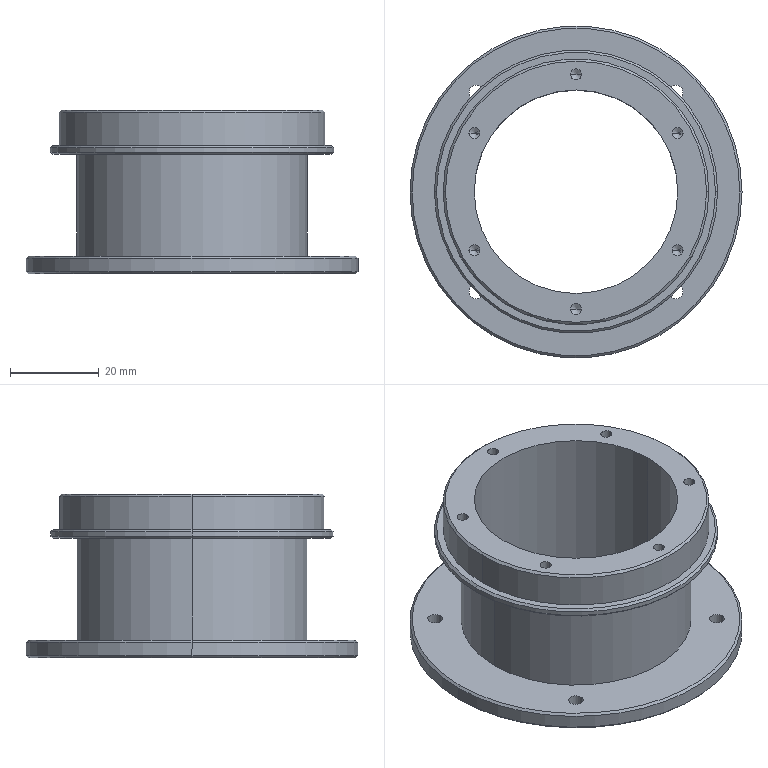Part | SolidWorks | features BaseBody 1 | 1 solid | 57 faces | box 75 x 75 x 37 mm | volume 33627 mm3 | cylinder 30 | cone 22 | plane 5 | commonest cylinder face diameters 2.5 x12 3.3 x8 46 x2 52 x2 60 x2 64 x2
STEP:
#1=CARTESIAN_POINT('',(23.,0.,10.));
#2=VERTEX_POINT('',#1);
#3=CARTESIAN_POINT('',(-23.,0.,10.));
#4=VERTEX_POINT('',#3);
#5=CARTESIAN_POINT('',(0.,0.,10.));
#6=DIRECTION('',(0.,0.,-1.));
#7=DIRECTION('',(-1.,0.,0.));
#8=AXIS2_PLACEMENT_3D('',#5,#6,#7);
#9=CIRCLE('',#8,23.);
#10=EDGE_CURVE('',#2,#4,#9,.T.);
#11=ORIENTED_EDGE('',*,*,#10,.F.);
#12=CARTESIAN_POINT('',(23.,0.,-27.));
#13=VERTEX_POINT('',#12);
#14=CARTESIAN_POINT('',(23.,0.,10.));
#15=DIRECTION('',(0.,0.,-1.));
#16=VECTOR('',#15,1000.);
#17=LINE('',#14,#16);
#18=EDGE_CURVE('',#2,#13,#17,.T.);
#19=ORIENTED_EDGE('',*,*,#18,.T.);
#20=CARTESIAN_POINT('',(-23.,0.,-27.));
#21=VERTEX_POINT('',#20);
#22=CARTESIAN_POINT('',(0.,0.,-27.));
#23=DIRECTION('',(0.,0.,1.));
#24=DIRECTION('',(-1.,0.,0.));
#25=AXIS2_PLACEMENT_3D('',#22,#23,#24);
#26=CIRCLE('',#25,23.);
#27=EDGE_CURVE('',#21,#13,#26,.T.);
#28=ORIENTED_EDGE('',*,*,#27,.F.);
#29=CARTESIAN_POINT('',(-23.,0.,10.));
#30=DIRECTION('',(0.,0.,-1.));
#31=VECTOR('',#30,1000.);
#32=LINE('',#29,#31);
#33=EDGE_CURVE('',#4,#21,#32,.T.);
#34=ORIENTED_EDGE('',*,*,#33,.F.);
#35=EDGE_LOOP('',(#11,#19,#28,#34));
#36=FACE_OUTER_BOUND('',#35,.T.);
#37=CARTESIAN_POINT('',(0.,0.,10.));
#38=DIRECTION('',(0.,0.,-1.));
#39=DIRECTION('',(-1.,0.,0.));
#40=AXIS2_PLACEMENT_3D('',#37,#38,#39);
#41=CYLINDRICAL_SURFACE('',#40,23.);
#42=ADVANCED_FACE('',(#36),#41,.F.);
#43=CARTESIAN_POINT('',(-24.2,-13.25,4.));
#44=VERTEX_POINT('',#43);
#45=CARTESIAN_POINT('',(-21.7,-13.25,4.));
#46=VERTEX_POINT('',#45);
#47=CARTESIAN_POINT('',(-22.95,-13.25,4.));
#48=DIRECTION('',(0.,0.,1.));
#49=DIRECTION('',(1.,0.,0.));
#50=AXIS2_PLACEMENT_3D('',#47,#48,#49);
#51=CIRCLE('',#50,1.25);
#52=EDGE_CURVE('',#44,#46,#51,.T.);
#53=ORIENTED_EDGE('',*,*,#52,.F.);
#54=CARTESIAN_POINT('',(-24.2,-13.25,10.));
#55=VERTEX_POINT('',#54);
#56=CARTESIAN_POINT('',(-24.2,-13.25,10.));
#57=DIRECTION('',(0.,0.,1.));
#58=VECTOR('',#57,1000.);
#59=LINE('',#56,#58);
#60=EDGE_CURVE('',#44,#55,#59,.T.);
#61=ORIENTED_EDGE('',*,*,#60,.T.);
#62=CARTESIAN_POINT('',(-21.7,-13.25,10.));
#63=VERTEX_POINT('',#62);
#64=CARTESIAN_POINT('',(-22.95,-13.25,10.));
#65=DIRECTION('',(0.,0.,-1.));
#66=DIRECTION('',(1.,0.,0.));
#67=AXIS2_PLACEMENT_3D('',#64,#65,#66);
#68=CIRCLE('',#67,1.25);
#69=EDGE_CURVE('',#63,#55,#68,.T.);
#70=ORIENTED_EDGE('',*,*,#69,.F.);
#71=CARTESIAN_POINT('',(-21.7,-13.25,10.));
#72=DIRECTION('',(0.,0.,1.));
#73=VECTOR('',#72,1000.);
#74=LINE('',#71,#73);
#75=EDGE_CURVE('',#46,#63,#74,.T.);
#76=ORIENTED_EDGE('',*,*,#75,.F.);
#77=EDGE_LOOP('',(#53,#61,#70,#76));
#78=FACE_OUTER_BOUND('',#77,.T.);
#79=CARTESIAN_POINT('',(-22.95,-13.25,10.));
#80=DIRECTION('',(0.,0.,1.));
#81=DIRECTION('',(1.,0.,0.));
#82=AXIS2_PLACEMENT_3D('',#79,#80,#81);
#83=CYLINDRICAL_SURFACE('',#82,1.25);
#84=ADVANCED_FACE('',(#78),#83,.F.);
#85=CARTESIAN_POINT('',(-24.2,13.25,4.));
#86=VERTEX_POINT('',#85);
#87=CARTESIAN_POINT('',(-21.7,13.25,4.));
#88=VERTEX_POINT('',#87);
#89=CARTESIAN_POINT('',(-22.95,13.25,4.));
#90=DIRECTION('',(0.,0.,1.));
#91=DIRECTION('',(1.,0.,0.));
#92=AXIS2_PLACEMENT_3D('',#89,#90,#91);
#93=CIRCLE('',#92,1.25);
#94=EDGE_CURVE('',#86,#88,#93,.T.);
#95=ORIENTED_EDGE('',*,*,#94,.F.);
#96=CARTESIAN_POINT('',(-24.2,13.25,10.));
#97=VERTEX_POINT('',#96);
#98=CARTESIAN_POINT('',(-24.2,13.25,10.));
#99=DIRECTION('',(0.,0.,1.));
#100=VECTOR('',#99,1000.);
#101=LINE('',#98,#100);
#102=EDGE_CURVE('',#86,#97,#101,.T.);
#103=ORIENTED_EDGE('',*,*,#102,.T.);
#104=CARTESIAN_POINT('',(-21.7,13.25,10.));
#105=VERTEX_POINT('',#104);
#106=CARTESIAN_POINT('',(-22.95,13.25,10.));
#107=DIRECTION('',(0.,0.,-1.));
#108=DIRECTION('',(1.,0.,0.));
#109=AXIS2_PLACEMENT_3D('',#106,#107,#108);
#110=CIRCLE('',#109,1.25);
#111=EDGE_CURVE('',#105,#97,#110,.T.);
#112=ORIENTED_EDGE('',*,*,#111,.F.);
#113=CARTESIAN_POINT('',(-21.7,13.25,10.));
#114=DIRECTION('',(0.,0.,1.));
#115=VECTOR('',#114,1000.);
#116=LINE('',#113,#115);
#117=EDGE_CURVE('',#88,#105,#116,.T.);
#118=ORIENTED_EDGE('',*,*,#117,.F.);
#119=EDGE_LOOP('',(#95,#103,#112,#118));
#120=FACE_OUTER_BOUND('',#119,.T.);
#121=CARTESIAN_POINT('',(-22.95,13.25,10.));
#122=DIRECTION('',(0.,0.,1.));
#123=DIRECTION('',(1.,0.,0.));
#124=AXIS2_PLACEMENT_3D('',#121,#122,#123);
#125=CYLINDRICAL_SURFACE('',#124,1.25);
#126=ADVANCED_FACE('',(#120),#125,.F.);
#127=CARTESIAN_POINT('',(-1.25,26.5,4.));
#128=VERTEX_POINT('',#127);
#129=CARTESIAN_POINT('',(1.25,26.5,4.));
#130=VERTEX_POINT('',#129);
#131=CARTESIAN_POINT('',(0.,26.5,4.));
#132=DIRECTION('',(0.,0.,1.));
#133=DIRECTION('',(1.,0.,0.));
#134=AXIS2_PLACEMENT_3D('',#131,#132,#133);
#135=CIRCLE('',#134,1.25);
#136=EDGE_CURVE('',#128,#130,#135,.T.);
#137=ORIENTED_EDGE('',*,*,#136,.F.);
#138=CARTESIAN_POINT('',(-1.25,26.5,10.));
#139=VERTEX_POINT('',#138);
#140=CARTESIAN_POINT('',(-1.25,26.5,10.));
#141=DIRECTION('',(0.,0.,1.));
#142=VECTOR('',#141,1000.);
#143=LINE('',#140,#142);
#144=EDGE_CURVE('',#128,#139,#143,.T.);
#145=ORIENTED_EDGE('',*,*,#144,.T.);
#146=CARTESIAN_POINT('',(1.25,26.5,10.));
#147=VERTEX_POINT('',#146);
#148=CARTESIAN_POINT('',(0.,26.5,10.));
#149=DIRECTION('',(0.,0.,-1.));
#150=DIRECTION('',(1.,0.,0.));
#151=AXIS2_PLACEMENT_3D('',#148,#149,#150);
#152=CIRCLE('',#151,1.25);
#153=EDGE_CURVE('',#147,#139,#152,.T.);
#154=ORIENTED_EDGE('',*,*,#153,.F.);
#155=CARTESIAN_POINT('',(1.25,26.5,10.));
#156=DIRECTION('',(0.,0.,1.));
#157=VECTOR('',#156,1000.);
#158=LINE('',#155,#157);
#159=EDGE_CURVE('',#130,#147,#158,.T.);
#160=ORIENTED_EDGE('',*,*,#159,.F.);
#161=EDGE_LOOP('',(#137,#145,#154,#160));
#162=FACE_OUTER_BOUND('',#161,.T.);
#163=CARTESIAN_POINT('',(0.,26.5,10.));
#164=DIRECTION('',(0.,0.,1.));
#165=DIRECTION('',(1.,0.,0.));
#166=AXIS2_PLACEMENT_3D('',#163,#164,#165);
#167=CYLINDRICAL_SURFACE('',#166,1.25);
#168=ADVANCED_FACE('',(#162),#167,.F.);
#169=CARTESIAN_POINT('',(21.7,13.25,4.));
#170=VERTEX_POINT('',#169);
#171=CARTESIAN_POINT('',(24.2,13.25,4.));
#172=VERTEX_POINT('',#171);
#173=CARTESIAN_POINT('',(22.95,13.25,4.));
#174=DIRECTION('',(0.,0.,1.));
#175=DIRECTION('',(1.,0.,0.));
#176=AXIS2_PLACEMENT_3D('',#173,#174,#175);
#177=CIRCLE('',#176,1.25);
#178=EDGE_CURVE('',#170,#172,#177,.T.);
#179=ORIENTED_EDGE('',*,*,#178,.F.);
#180=CARTESIAN_POINT('',(21.7,13.25,10.));
#181=VERTEX_POINT('',#180);
#182=CARTESIAN_POINT('',(21.7,13.25,10.));
#183=DIRECTION('',(0.,0.,1.));
#184=VECTOR('',#183,1000.);
#185=LINE('',#182,#184);
#186=EDGE_CURVE('',#170,#181,#185,.T.);
#187=ORIENTED_EDGE('',*,*,#186,.T.);
#188=CARTESIAN_POINT('',(24.2,13.25,10.));
#189=VERTEX_POINT('',#188);
#190=CARTESIAN_POINT('',(22.95,13.25,10.));
#191=DIRECTION('',(0.,0.,-1.));
#192=DIRECTION('',(1.,0.,0.));
#193=AXIS2_PLACEMENT_3D('',#190,#191,#192);
#194=CIRCLE('',#193,1.25);
#195=EDGE_CURVE('',#189,#181,#194,.T.);
#196=ORIENTED_EDGE('',*,*,#195,.F.);
#197=CARTESIAN_POINT('',(24.2,13.25,10.));
#198=DIRECTION('',(0.,0.,1.));
#199=VECTOR('',#198,1000.);
#200=LINE('',#197,#199);
#201=EDGE_CURVE('',#172,#189,#200,.T.);
#202=ORIENTED_EDGE('',*,*,#201,.F.);
#203=EDGE_LOOP('',(#179,#187,#196,#202));
#204=FACE_OUTER_BOUND('',#203,.T.);
#205=CARTESIAN_POINT('',(22.95,13.25,10.));
#206=DIRECTION('',(0.,0.,1.));
#207=DIRECTION('',(1.,0.,0.));
#208=AXIS2_PLACEMENT_3D('',#205,#206,#207);
#209=CYLINDRICAL_SURFACE('',#208,1.25);
#210=ADVANCED_FACE('',(#204),#209,.F.);
#211=CARTESIAN_POINT('',(21.7,-13.25,4.));
#212=VERTEX_POINT('',#211);
#213=CARTESIAN_POINT('',(24.2,-13.25,4.));
#214=VERTEX_POINT('',#213);
#215=CARTESIAN_POINT('',(22.95,-13.25,4.));
#216=DIRECTION('',(0.,0.,1.));
#217=DIRECTION('',(1.,0.,0.));
#218=AXIS2_PLACEMENT_3D('',#215,#216,#217);
#219=CIRCLE('',#218,1.25);
#220=EDGE_CURVE('',#212,#214,#219,.T.);
#221=ORIENTED_EDGE('',*,*,#220,.F.);
#222=CARTESIAN_POINT('',(21.7,-13.25,10.));
#223=VERTEX_POINT('',#222);
#224=CARTESIAN_POINT('',(21.7,-13.25,10.));
#225=DIRECTION('',(0.,0.,1.));
#226=VECTOR('',#225,1000.);
#227=LINE('',#224,#226);
#228=EDGE_CURVE('',#212,#223,#227,.T.);
#229=ORIENTED_EDGE('',*,*,#228,.T.);
#230=CARTESIAN_POINT('',(24.2,-13.25,10.));
#231=VERTEX_POINT('',#230);
#232=CARTESIAN_POINT('',(22.95,-13.25,10.));
#233=DIRECTION('',(0.,0.,-1.));
#234=DIRECTION('',(1.,0.,0.));
#235=AXIS2_PLACEMENT_3D('',#232,#233,#234);
#236=CIRCLE('',#235,1.25);
#237=EDGE_CURVE('',#231,#223,#236,.T.);
#238=ORIENTED_EDGE('',*,*,#237,.F.);
#239=CARTESIAN_POINT('',(24.2,-13.25,10.));
#240=DIRECTION('',(0.,0.,1.));
#241=VECTOR('',#240,1000.);
#242=LINE('',#239,#241);
#243=EDGE_CURVE('',#214,#231,#242,.T.);
#244=ORIENTED_EDGE('',*,*,#243,.F.);
#245=EDGE_LOOP('',(#221,#229,#238,#244));
#246=FACE_OUTER_BOUND('',#245,.T.);
#247=CARTESIAN_POINT('',(22.95,-13.25,10.));
#248=DIRECTION('',(0.,0.,1.));
#249=DIRECTION('',(1.,0.,0.));
#250=AXIS2_PLACEMENT_3D('',#247,#248,#249);
#251=CYLINDRICAL_SURFACE('',#250,1.25);
#252=ADVANCED_FACE('',(#246),#251,.F.);
#253=CARTESIAN_POINT('',(-1.25,-26.5,4.));
#254=VERTEX_POINT('',#253);
#255=CARTESIAN_POINT('',(1.25,-26.5,4.));
#256=VERTEX_POINT('',#255);
#257=CARTESIAN_POINT('',(0.,-26.5,4.));
#258=DIRECTION('',(0.,0.,1.));
#259=DIRECTION('',(1.,0.,0.));
#260=AXIS2_PLACEMENT_3D('',#257,#258,#259);
#261=CIRCLE('',#260,1.25);
#262=EDGE_CURVE('',#254,#256,#261,.T.);
#263=ORIENTED_EDGE('',*,*,#262,.F.);
#264=CARTESIAN_POINT('',(-1.25,-26.5,10.));
#265=VERTEX_POINT('',#264);
#266=CARTESIAN_POINT('',(-1.25,-26.5,10.));
#267=DIRECTION('',(0.,0.,1.));
#268=VECTOR('',#267,1000.);
#269=LINE('',#266,#268);
#270=EDGE_CURVE('',#254,#265,#269,.T.);
#271=ORIENTED_EDGE('',*,*,#270,.T.);
#272=CARTESIAN_POINT('',(1.25,-26.5,10.));
#273=VERTEX_POINT('',#272);
#274=CARTESIAN_POINT('',(0.,-26.5,10.));
#275=DIRECTION('',(0.,0.,-1.));
#276=DIRECTION('',(1.,0.,0.));
#277=AXIS2_PLACEMENT_3D('',#274,#275,#276);
#278=CIRCLE('',#277,1.25);
#279=EDGE_CURVE('',#273,#265,#278,.T.);
#280=ORIENTED_EDGE('',*,*,#279,.F.);
#281=CARTESIAN_POINT('',(1.25,-26.5,10.));
#282=DIRECTION('',(0.,0.,1.));
#283=VECTOR('',#282,1000.);
#284=LINE('',#281,#283);
#285=EDGE_CURVE('',#256,#273,#284,.T.);
#286=ORIENTED_EDGE('',*,*,#285,.F.);
#287=EDGE_LOOP('',(#263,#271,#280,#286));
#288=FACE_OUTER_BOUND('',#287,.T.);
#289=CARTESIAN_POINT('',(0.,-26.5,10.));
#290=DIRECTION('',(0.,0.,1.));
#291=DIRECTION('',(1.,0.,0.));
#292=AXIS2_PLACEMENT_3D('',#289,#290,#291);
#293=CYLINDRICAL_SURFACE('',#292,1.25);
#294=ADVANCED_FACE('',(#288),#293,.F.);
#295=CARTESIAN_POINT('',(29.5,0.,10.));
#296=VERTEX_POINT('',#295);
#297=CARTESIAN_POINT('',(-29.5,0.,10.));
#298=VERTEX_POINT('',#297);
#299=CARTESIAN_POINT('',(0.,0.,10.));
#300=DIRECTION('',(0.,0.,1.));
#301=DIRECTION('',(-1.,0.,0.));
#302=AXIS2_PLACEMENT_3D('',#299,#300,#301);
#303=CIRCLE('',#302,29.5);
#304=EDGE_CURVE('',#296,#298,#303,.T.);
#305=ORIENTED_EDGE('',*,*,#304,.F.);
#306=CARTESIAN_POINT('',(30.,0.,9.5));
#307=VERTEX_POINT('',#306);
#308=CARTESIAN_POINT('',(30.,0.,9.5));
#309=DIRECTION('',(0.7071,0.,-0.7071));
#310=VECTOR('',#309,1000.);
#311=LINE('',#308,#310);
#312=EDGE_CURVE('',#296,#307,#311,.T.);
#313=ORIENTED_EDGE('',*,*,#312,.T.);
#314=CARTESIAN_POINT('',(-30.,0.,9.5));
#315=VERTEX_POINT('',#314);
#316=CARTESIAN_POINT('',(0.,0.,9.5));
#317=DIRECTION('',(0.,0.,1.));
#318=DIRECTION('',(-1.,0.,0.));
#319=AXIS2_PLACEMENT_3D('',#316,#317,#318);
#320=CIRCLE('',#319,30.);
#321=EDGE_CURVE('',#307,#315,#320,.T.);
#322=ORIENTED_EDGE('',*,*,#321,.T.);
#323=CARTESIAN_POINT('',(-30.,0.,9.5));
#324=DIRECTION('',(-0.7071,0.,-0.7071));
#325=VECTOR('',#324,1000.);
#326=LINE('',#323,#325);
#327=EDGE_CURVE('',#298,#315,#326,.T.);
#328=ORIENTED_EDGE('',*,*,#327,.F.);
#329=EDGE_LOOP('',(#305,#313,#322,#328));
#330=FACE_OUTER_BOUND('',#329,.T.);
#331=CARTESIAN_POINT('',(0.,0.,9.5));
#332=DIRECTION('',(0.,0.,-1.));
#333=DIRECTION('',(-1.,0.,0.));
#334=AXIS2_PLACEMENT_3D('',#331,#332,#333);
#335=CONICAL_SURFACE('',#334,30.,0.7854);
#336=ADVANCED_FACE('',(#330),#335,.T.);
#337=CARTESIAN_POINT('',(24.15,22.5,-23.));
#338=VERTEX_POINT('',#337);
#339=CARTESIAN_POINT('',(20.85,22.5,-23.));
#340=VERTEX_POINT('',#339);
#341=CARTESIAN_POINT('',(22.5,22.5,-23.));
#342=DIRECTION('',(0.,0.,-1.));
#343=DIRECTION('',(-1.,0.,0.));
#344=AXIS2_PLACEMENT_3D('',#341,#342,#343);
#345=CIRCLE('',#344,1.65);
#346=EDGE_CURVE('',#338,#340,#345,.T.);
#347=ORIENTED_EDGE('',*,*,#346,.F.);
#348=CARTESIAN_POINT('',(24.15,22.5,-27.));
#349=VERTEX_POINT('',#348);
#350=CARTESIAN_POINT('',(24.15,22.5,-27.));
#351=DIRECTION('',(0.,0.,-1.));
#352=VECTOR('',#351,1000.);
#353=LINE('',#350,#352);
#354=EDGE_CURVE('',#338,#349,#353,.T.);
#355=ORIENTED_EDGE('',*,*,#354,.T.);
#356=CARTESIAN_POINT('',(20.85,22.5,-27.));
#357=VERTEX_POINT('',#356);
#358=CARTESIAN_POINT('',(22.5,22.5,-27.));
#359=DIRECTION('',(0.,0.,1.));
#360=DIRECTION('',(-1.,0.,0.));
#361=AXIS2_PLACEMENT_3D('',#358,#359,#360);
#362=CIRCLE('',#361,1.65);
#363=EDGE_CURVE('',#357,#349,#362,.T.);
#364=ORIENTED_EDGE('',*,*,#363,.F.);
#365=CARTESIAN_POINT('',(20.85,22.5,-27.));
#366=DIRECTION('',(0.,0.,-1.));
#367=VECTOR('',#366,1000.);
#368=LINE('',#365,#367);
#369=EDGE_CURVE('',#340,#357,#368,.T.);
#370=ORIENTED_EDGE('',*,*,#369,.F.);
#371=EDGE_LOOP('',(#347,#355,#364,#370));
#372=FACE_OUTER_BOUND('',#371,.T.);
#373=CARTESIAN_POINT('',(22.5,22.5,-27.));
#374=DIRECTION('',(0.,0.,-1.));
#375=DIRECTION('',(-1.,0.,0.));
#376=AXIS2_PLACEMENT_3D('',#373,#374,#375);
#377=CYLINDRICAL_SURFACE('',#376,1.65);
#378=ADVANCED_FACE('',(#372),#377,.F.);
#379=CARTESIAN_POINT('',(24.15,-22.5,-23.));
#380=VERTEX_POINT('',#379);
#381=CARTESIAN_POINT('',(20.85,-22.5,-23.));
#382=VERTEX_POINT('',#381);
#383=CARTESIAN_POINT('',(22.5,-22.5,-23.));
#384=DIRECTION('',(0.,0.,-1.));
#385=DIRECTION('',(-1.,0.,0.));
#386=AXIS2_PLACEMENT_3D('',#383,#384,#385);
#387=CIRCLE('',#386,1.65);
#388=EDGE_CURVE('',#380,#382,#387,.T.);
#389=ORIENTED_EDGE('',*,*,#388,.F.);
#390=CARTESIAN_POINT('',(24.15,-22.5,-27.));
#391=VERTEX_POINT('',#390);
#392=CARTESIAN_POINT('',(24.15,-22.5,-27.));
#393=DIRECTION('',(0.,0.,-1.));
#394=VECTOR('',#393,1000.);
#395=LINE('',#392,#394);
#396=EDGE_CURVE('',#380,#391,#395,.T.);
#397=ORIENTED_EDGE('',*,*,#396,.T.);
#398=CARTESIAN_POINT('',(20.85,-22.5,-27.));
#399=VERTEX_POINT('',#398);
#400=CARTESIAN_POINT('',(22.5,-22.5,-27.));
#401=DIRECTION('',(0.,0.,1.));
#402=DIRECTION('',(-1.,0.,0.));
#403=AXIS2_PLACEMENT_3D('',#400,#401,#402);
#404=CIRCLE('',#403,1.65);
#405=EDGE_CURVE('',#399,#391,#404,.T.);
#406=ORIENTED_EDGE('',*,*,#405,.F.);
#407=CARTESIAN_POINT('',(20.85,-22.5,-27.));
#408=DIRECTION('',(0.,0.,-1.));
#409=VECTOR('',#408,1000.);
#410=LINE('',#407,#409);
#411=EDGE_CURVE('',#382,#399,#410,.T.);
#412=ORIENTED_EDGE('',*,*,#411,.F.);
#413=EDGE_LOOP('',(#389,#397,#406,#412));
#414=FACE_OUTER_BOUND('',#413,.T.);
#415=CARTESIAN_POINT('',(22.5,-22.5,-27.));
#416=DIRECTION('',(0.,0.,-1.));
#417=DIRECTION('',(-1.,0.,0.));
#418=AXIS2_PLACEMENT_3D('',#415,#416,#417);
#419=CYLINDRICAL_SURFACE('',#418,1.65);
#420=ADVANCED_FACE('',(#414),#419,.F.);
#421=CARTESIAN_POINT('',(-20.85,22.5,-23.));
#422=VERTEX_POINT('',#421);
#423=CARTESIAN_POINT('',(-24.15,22.5,-23.));
#424=VERTEX_POINT('',#423);
#425=CARTESIAN_POINT('',(-22.5,22.5,-23.));
#426=DIRECTION('',(0.,0.,-1.));
#427=DIRECTION('',(-1.,0.,0.));
#428=AXIS2_PLACEMENT_3D('',#425,#426,#427);
#429=CIRCLE('',#428,1.65);
#430=EDGE_CURVE('',#422,#424,#429,.T.);
#431=ORIENTED_EDGE('',*,*,#430,.F.);
#432=CARTESIAN_POINT('',(-20.85,22.5,-27.));
#433=VERTEX_POINT('',#432);
#434=CARTESIAN_POINT('',(-20.85,22.5,-27.));
#435=DIRECTION('',(0.,0.,-1.));
#436=VECTOR('',#435,1000.);
#437=LINE('',#434,#436);
#438=EDGE_CURVE('',#422,#433,#437,.T.);
#439=ORIENTED_EDGE('',*,*,#438,.T.);
#440=CARTESIAN_POINT('',(-24.15,22.5,-27.));
#441=VERTEX_POINT('',#440);
#442=CARTESIAN_POINT('',(-22.5,22.5,-27.));
#443=DIRECTION('',(0.,0.,1.));
#444=DIRECTION('',(-1.,0.,0.));
#445=AXIS2_PLACEMENT_3D('',#442,#443,#444);
#446=CIRCLE('',#445,1.65);
#447=EDGE_CURVE('',#441,#433,#446,.T.);
#448=ORIENTED_EDGE('',*,*,#447,.F.);
#449=CARTESIAN_POINT('',(-24.15,22.5,-27.));
#450=DIRECTION('',(0.,0.,-1.));
#451=VECTOR('',#450,1000.);
#452=LINE('',#449,#451);
#453=EDGE_CURVE('',#424,#441,#452,.T.);
#454=ORIENTED_EDGE('',*,*,#453,.F.);
#455=EDGE_LOOP('',(#431,#439,#448,#454));
#456=FACE_OUTER_BOUND('',#455,.T.);
#457=CARTESIAN_POINT('',(-22.5,22.5,-27.));
#458=DIRECTION('',(0.,0.,-1.));
#459=DIRECTION('',(-1.,0.,0.));
#460=AXIS2_PLACEMENT_3D('',#457,#458,#459);
#461=CYLINDRICAL_SURFACE('',#460,1.65);
#462=ADVANCED_FACE('',(#456),#461,.F.);
#463=CARTESIAN_POINT('',(-20.85,-22.5,-23.));
#464=VERTEX_POINT('',#463);
#465=CARTESIAN_POINT('',(-24.15,-22.5,-23.));
#466=VERTEX_POINT('',#465);
#467=CARTESIAN_POINT('',(-22.5,-22.5,-23.));
#468=DIRECTION('',(0.,0.,-1.));
#469=DIRECTION('',(-1.,0.,0.));
#470=AXIS2_PLACEMENT_3D('',#467,#468,#469);
#471=CIRCLE('',#470,1.65);
#472=EDGE_CURVE('',#464,#466,#471,.T.);
#473=ORIENTED_EDGE('',*,*,#472,.F.);
#474=CARTESIAN_POINT('',(-20.85,-22.5,-27.));
#475=VERTEX_POINT('',#474);
#476=CARTESIAN_POINT('',(-20.85,-22.5,-27.));
#477=DIRECTION('',(0.,0.,-1.));
#478=VECTOR('',#477,1000.);
#479=LINE('',#476,#478);
#480=EDGE_CURVE('',#464,#475,#479,.T.);
#481=ORIENTED_EDGE('',*,*,#480,.T.);
#482=CARTESIAN_POINT('',(-24.15,-22.5,-27.));
#483=VERTEX_POINT('',#482);
#484=CARTESIAN_POINT('',(-22.5,-22.5,-27.));
#485=DIRECTION('',(0.,0.,1.));
#486=DIRECTION('',(-1.,0.,0.));
#487=AXIS2_PLACEMENT_3D('',#484,#485,#486);
#488=CIRCLE('',#487,1.65);
#489=EDGE_CURVE('',#483,#475,#488,.T.);
#490=ORIENTED_EDGE('',*,*,#489,.F.);
#491=CARTESIAN_POINT('',(-24.15,-22.5,-27.));
#492=DIRECTION('',(0.,0.,-1.));
#493=VECTOR('',#492,1000.);
#494=LINE('',#491,#493);
#495=EDGE_CURVE('',#466,#483,#494,.T.);
#496=ORIENTED_EDGE('',*,*,#495,.F.);
#497=EDGE_LOOP('',(#473,#481,#490,#496));
#498=FACE_OUTER_BOUND('',#497,.T.);
#499=CARTESIAN_POINT('',(-22.5,-22.5,-27.));
#500=DIRECTION('',(0.,0.,-1.));
#501=DIRECTION('',(-1.,0.,0.));
#502=AXIS2_PLACEMENT_3D('',#499,#500,#501);
#503=CYLINDRICAL_SURFACE('',#502,1.65);
#504=ADVANCED_FACE('',(#498),#503,.F.);
#505=CARTESIAN_POINT('',(-37.,0.,-27.));
#506=VERTEX_POINT('',#505);
#507=CARTESIAN_POINT('',(37.,0.,-27.));
#508=VERTEX_POINT('',#507);
#509=CARTESIAN_POINT('',(0.,0.,-27.));
#510=DIRECTION('',(0.,0.,-1.));
#511=DIRECTION('',(1.,0.,0.));
#512=AXIS2_PLACEMENT_3D('',#509,#510,#511);
#513=CIRCLE('',#512,37.);
#514=EDGE_CURVE('',#506,#508,#513,.T.);
#515=ORIENTED_EDGE('',*,*,#514,.F.);
#516=CARTESIAN_POINT('',(-37.5,0.,-26.5));
#517=VERTEX_POINT('',#516);
#518=CARTESIAN_POINT('',(-37.5,0.,-26.5));
#519=DIRECTION('',(-0.7071,0.,0.7071));
#520=VECTOR('',#519,1000.);
#521=LINE('',#518,#520);
#522=EDGE_CURVE('',#506,#517,#521,.T.);
#523=ORIENTED_EDGE('',*,*,#522,.T.);
#524=CARTESIAN_POINT('',(37.5,0.,-26.5));
#525=VERTEX_POINT('',#524);
#526=CARTESIAN_POINT('',(0.,0.,-26.5));
#527=DIRECTION('',(0.,0.,-1.));
#528=DIRECTION('',(1.,0.,0.));
#529=AXIS2_PLACEMENT_3D('',#526,#527,#528);
#530=CIRCLE('',#529,37.5);
#531=EDGE_CURVE('',#517,#525,#530,.T.);
#532=ORIENTED_EDGE('',*,*,#531,.T.);
#533=CARTESIAN_POINT('',(37.5,0.,-26.5));
#534=DIRECTION('',(0.7071,0.,0.7071));
#535=VECTOR('',#534,1000.);
#536=LINE('',#533,#535);
#537=EDGE_CURVE('',#508,#525,#536,.T.);
#538=ORIENTED_EDGE('',*,*,#537,.F.);
#539=EDGE_LOOP('',(#515,#523,#532,#538));
#540=FACE_OUTER_BOUND('',#539,.T.);
#541=CARTESIAN_POINT('',(0.,0.,-26.5));
#542=DIRECTION('',(0.,0.,1.));
#543=DIRECTION('',(1.,0.,0.));
#544=AXIS2_PLACEMENT_3D('',#541,#542,#543);
#545=CONICAL_SURFACE('',#544,37.5,0.7854);
#546=ADVANCED_FACE('',(#540),#545,.T.);
#547=CARTESIAN_POINT('',(-22.95,-13.25,3.249));
#548=VERTEX_POINT('',#547);
#549=CARTESIAN_POINT('',(-21.7,-13.25,4.));
#550=DIRECTION('',(0.8572,0.,0.515));
#551=VECTOR('',#550,1000.);
#552=LINE('',#549,#551);
#553=EDGE_CURVE('',#548,#46,#552,.T.);
#554=ORIENTED_EDGE('',*,*,#553,.F.);
#555=CARTESIAN_POINT('',(-24.2,-13.25,4.));
#556=DIRECTION('',(-0.8572,0.,0.515));
#557=VECTOR('',#556,1000.);
#558=LINE('',#555,#557);
#559=EDGE_CURVE('',#548,#44,#558,.T.);
#560=ORIENTED_EDGE('',*,*,#559,.T.);
#561=ORIENTED_EDGE('',*,*,#52,.T.);
#562=EDGE_LOOP('',(#554,#560,#561));
#563=FACE_OUTER_BOUND('',#562,.T.);
#564=CARTESIAN_POINT('',(-22.95,-13.25,4.));
#565=DIRECTION('',(0.,0.,1.));
#566=DIRECTION('',(1.,0.,0.));
#567=AXIS2_PLACEMENT_3D('',#564,#565,#566);
#568=CONICAL_SURFACE('',#567,1.25,1.03);
#569=ADVANCED_FACE('',(#563),#568,.F.);
#570=CARTESIAN_POINT('',(-22.95,13.25,3.249));
#571=VERTEX_POINT('',#570);
#572=CARTESIAN_POINT('',(-21.7,13.25,4.));
#573=DIRECTION('',(0.8572,0.,0.515));
#574=VECTOR('',#573,1000.);
#575=LINE('',#572,#574);
#576=EDGE_CURVE('',#571,#88,#575,.T.);
#577=ORIENTED_EDGE('',*,*,#576,.F.);
#578=CARTESIAN_POINT('',(-24.2,13.25,4.));
#579=DIRECTION('',(-0.8572,0.,0.515));
#580=VECTOR('',#579,1000.);
#581=LINE('',#578,#580);
#582=EDGE_CURVE('',#571,#86,#581,.T.);
#583=ORIENTED_EDGE('',*,*,#582,.T.);
#584=ORIENTED_EDGE('',*,*,#94,.T.);
#585=EDGE_LOOP('',(#577,#583,#584));
#586=FACE_OUTER_BOUND('',#585,.T.);
#587=CARTESIAN_POINT('',(-22.95,13.25,4.));
#588=DIRECTION('',(0.,0.,1.));
#589=DIRECTION('',(1.,0.,0.));
#590=AXIS2_PLACEMENT_3D('',#587,#588,#589);
#591=CONICAL_SURFACE('',#590,1.25,1.03);
#592=ADVANCED_FACE('',(#586),#591,.F.);
#593=CARTESIAN_POINT('',(0.,26.5,3.249));
#594=VERTEX_POINT('',#593);
#595=CARTESIAN_POINT('',(1.25,26.5,4.));
#596=DIRECTION('',(0.8572,0.,0.515));
#597=VECTOR('',#596,1000.);
#598=LINE('',#595,#597);
#599=EDGE_CURVE('',#594,#130,#598,.T.);
#600=ORIENTED_EDGE('',*,*,#599,.F.);
#601=CARTESIAN_POINT('',(-1.25,26.5,4.));
#602=DIRECTION('',(-0.8572,0.,0.515));
#603=VECTOR('',#602,1000.);
#604=LINE('',#601,#603);
#605=EDGE_CURVE('',#594,#128,#604,.T.);
#606=ORIENTED_EDGE('',*,*,#605,.T.);
#607=ORIENTED_EDGE('',*,*,#136,.T.);
#608=EDGE_LOOP('',(#600,#606,#607));
#609=FACE_OUTER_BOUND('',#608,.T.);
#610=CARTESIAN_POINT('',(0.,26.5,4.));
#611=DIRECTION('',(0.,0.,1.));
#612=DIRECTION('',(1.,0.,0.));
#613=AXIS2_PLACEMENT_3D('',#610,#611,#612);
#614=CONICAL_SURFACE('',#613,1.25,1.03);
#615=ADVANCED_FACE('',(#609),#614,.F.);
#616=CARTESIAN_POINT('',(22.95,13.25,3.249));
#617=VERTEX_POINT('',#616);
#618=CARTESIAN_POINT('',(24.2,13.25,4.));
#619=DIRECTION('',(0.8572,0.,0.515));
#620=VECTOR('',#619,1000.);
#621=LINE('',#618,#620);
#622=EDGE_CURVE('',#617,#172,#621,.T.);
#623=ORIENTED_EDGE('',*,*,#622,.F.);
#624=CARTESIAN_POINT('',(21.7,13.25,4.));
#625=DIRECTION('',(-0.8572,0.,0.515));
#626=VECTOR('',#625,1000.);
#627=LINE('',#624,#626);
#628=EDGE_CURVE('',#617,#170,#627,.T.);
#629=ORIENTED_EDGE('',*,*,#628,.T.);
#630=ORIENTED_EDGE('',*,*,#178,.T.);
#631=EDGE_LOOP('',(#623,#629,#630));
#632=FACE_OUTER_BOUND('',#631,.T.);
#633=CARTESIAN_POINT('',(22.95,13.25,4.));
#634=DIRECTION('',(0.,0.,1.));
#635=DIRECTION('',(1.,0.,0.));
#636=AXIS2_PLACEMENT_3D('',#633,#634,#635);
#637=CONICAL_SURFACE('',#636,1.25,1.03);
#638=ADVANCED_FACE('',(#632),#637,.F.);
#639=CARTESIAN_POINT('',(22.95,-13.25,3.249));
#640=VERTEX_POINT('',#639);
#641=CARTESIAN_POINT('',(24.2,-13.25,4.));
#642=DIRECTION('',(0.8572,0.,0.515));
#643=VECTOR('',#642,1000.);
#644=LINE('',#641,#643);
#645=EDGE_CURVE('',#640,#214,#644,.T.);
#646=ORIENTED_EDGE('',*,*,#645,.F.);
#647=CARTESIAN_POINT('',(21.7,-13.25,4.));
#648=DIRECTION('',(-0.8572,0.,0.515));
#649=VECTOR('',#648,1000.);
#650=LINE('',#647,#649);
#651=EDGE_CURVE('',#640,#212,#650,.T.);
#652=ORIENTED_EDGE('',*,*,#651,.T.);
#653=ORIENTED_EDGE('',*,*,#220,.T.);
#654=EDGE_LOOP('',(#646,#652,#653));
#655=FACE_OUTER_BOUND('',#654,.T.);
#656=CARTESIAN_POINT('',(22.95,-13.25,4.));
#657=DIRECTION('',(0.,0.,1.));
#658=DIRECTION('',(1.,0.,0.));
#659=AXIS2_PLACEMENT_3D('',#656,#657,#658);
#660=CONICAL_SURFACE('',#659,1.25,1.03);
#661=ADVANCED_FACE('',(#655),#660,.F.);
#662=CARTESIAN_POINT('',(0.,-26.5,3.249));
#663=VERTEX_POINT('',#662);
#664=CARTESIAN_POINT('',(1.25,-26.5,4.));
#665=DIRECTION('',(0.8572,0.,0.515));
#666=VECTOR('',#665,1000.);
#667=LINE('',#664,#666);
#668=EDGE_CURVE('',#663,#256,#667,.T.);
#669=ORIENTED_EDGE('',*,*,#668,.F.);
#670=CARTESIAN_POINT('',(-1.25,-26.5,4.));
#671=DIRECTION('',(-0.8572,0.,0.515));
#672=VECTOR('',#671,1000.);
#673=LINE('',#670,#672);
#674=EDGE_CURVE('',#663,#254,#673,.T.);
#675=ORIENTED_EDGE('',*,*,#674,.T.);
#676=ORIENTED_EDGE('',*,*,#262,.T.);
#677=EDGE_LOOP('',(#669,#675,#676));
#678=FACE_OUTER_BOUND('',#677,.T.);
#679=CARTESIAN_POINT('',(0.,-26.5,4.));
#680=DIRECTION('',(0.,0.,1.));
#681=DIRECTION('',(1.,0.,0.));
#682=AXIS2_PLACEMENT_3D('',#679,#680,#681);
#683=CONICAL_SURFACE('',#682,1.25,1.03);
#684=ADVANCED_FACE('',(#678),#683,.F.);
#685=ORIENTED_EDGE('',*,*,#321,.F.);
#686=CARTESIAN_POINT('',(30.,0.,2.));
#687=VERTEX_POINT('',#686);
#688=CARTESIAN_POINT('',(30.,0.,10.));
#689=DIRECTION('',(0.,0.,-1.));
#690=VECTOR('',#689,1000.);
#691=LINE('',#688,#690);
#692=EDGE_CURVE('',#307,#687,#691,.T.);
#693=ORIENTED_EDGE('',*,*,#692,.T.);
#694=CARTESIAN_POINT('',(-30.,0.,2.));
#695=VERTEX_POINT('',#694);
#696=CARTESIAN_POINT('',(0.,0.,2.));
#697=DIRECTION('',(0.,0.,1.));
#698=DIRECTION('',(-1.,0.,0.));
#699=AXIS2_PLACEMENT_3D('',#696,#697,#698);
#700=CIRCLE('',#699,30.);
#701=EDGE_CURVE('',#687,#695,#700,.T.);
#702=ORIENTED_EDGE('',*,*,#701,.T.);
#703=CARTESIAN_POINT('',(-30.,0.,10.));
#704=DIRECTION('',(0.,0.,-1.));
#705=VECTOR('',#704,1000.);
#706=LINE('',#703,#705);
#707=EDGE_CURVE('',#315,#695,#706,.T.);
#708=ORIENTED_EDGE('',*,*,#707,.F.);
#709=EDGE_LOOP('',(#685,#693,#702,#708));
#710=FACE_OUTER_BOUND('',#709,.T.);
#711=CARTESIAN_POINT('',(0.,0.,10.));
#712=DIRECTION('',(0.,0.,-1.));
#713=DIRECTION('',(-1.,0.,0.));
#714=AXIS2_PLACEMENT_3D('',#711,#712,#713);
#715=CYLINDRICAL_SURFACE('',#714,30.);
#716=ADVANCED_FACE('',(#710),#715,.T.);
#717=ORIENTED_EDGE('',*,*,#531,.F.);
#718=CARTESIAN_POINT('',(-37.5,0.,-23.5));
#719=VERTEX_POINT('',#718);
#720=CARTESIAN_POINT('',(-37.5,0.,-27.));
#721=DIRECTION('',(0.,0.,1.));
#722=VECTOR('',#721,1000.);
#723=LINE('',#720,#722);
#724=EDGE_CURVE('',#517,#719,#723,.T.);
#725=ORIENTED_EDGE('',*,*,#724,.T.);
#726=CARTESIAN_POINT('',(37.5,0.,-23.5));
#727=VERTEX_POINT('',#726);
#728=CARTESIAN_POINT('',(0.,0.,-23.5));
#729=DIRECTION('',(0.,0.,-1.));
#730=DIRECTION('',(1.,0.,0.));
#731=AXIS2_PLACEMENT_3D('',#728,#729,#730);
#732=CIRCLE('',#731,37.5);
#733=EDGE_CURVE('',#719,#727,#732,.T.);
#734=ORIENTED_EDGE('',*,*,#733,.T.);
#735=CARTESIAN_POINT('',(37.5,0.,-27.));
#736=DIRECTION('',(0.,0.,1.));
#737=VECTOR('',#736,1000.);
#738=LINE('',#735,#737);
#739=EDGE_CURVE('',#525,#727,#738,.T.);
#740=ORIENTED_EDGE('',*,*,#739,.F.);
#741=EDGE_LOOP('',(#717,#725,#734,#740));
#742=FACE_OUTER_BOUND('',#741,.T.);
#743=CARTESIAN_POINT('',(0.,0.,-27.));
#744=DIRECTION('',(0.,0.,1.));
#745=DIRECTION('',(1.,0.,0.));
#746=AXIS2_PLACEMENT_3D('',#743,#744,#745);
#747=CYLINDRICAL_SURFACE('',#746,37.5);
#748=ADVANCED_FACE('',(#742),#747,.T.);
#749=CARTESIAN_POINT('',(26.,0.,-23.));
#750=VERTEX_POINT('',#749);
#751=CARTESIAN_POINT('',(-26.,0.,-23.));
#752=VERTEX_POINT('',#751);
#753=CARTESIAN_POINT('',(0.,0.,-23.));
#754=DIRECTION('',(0.,0.,1.));
#755=DIRECTION('',(1.,0.,0.));
#756=AXIS2_PLACEMENT_3D('',#753,#754,#755);
#757=CIRCLE('',#756,26.);
#758=EDGE_CURVE('',#750,#752,#757,.T.);
#759=ORIENTED_EDGE('',*,*,#758,.T.);
#760=CARTESIAN_POINT('',(-26.,0.,0.));
#761=VERTEX_POINT('',#760);
#762=CARTESIAN_POINT('',(-26.,0.,-23.));
#763=DIRECTION('',(0.,0.,1.));
#764=VECTOR('',#763,1000.);
#765=LINE('',#762,#764);
#766=EDGE_CURVE('',#752,#761,#765,.T.);
#767=ORIENTED_EDGE('',*,*,#766,.T.);
#768=CARTESIAN_POINT('',(26.,0.,0.));
#769=VERTEX_POINT('',#768);
#770=CARTESIAN_POINT('',(0.,0.,0.));
#771=DIRECTION('',(0.,0.,-1.));
#772=DIRECTION('',(1.,0.,0.));
#773=AXIS2_PLACEMENT_3D('',#770,#771,#772);
#774=CIRCLE('',#773,26.);
#775=EDGE_CURVE('',#761,#769,#774,.T.);
#776=ORIENTED_EDGE('',*,*,#775,.T.);
#777=CARTESIAN_POINT('',(26.,0.,-23.));
#778=DIRECTION('',(0.,0.,1.));
#779=VECTOR('',#778,1000.);
#780=LINE('',#777,#779);
#781=EDGE_CURVE('',#750,#769,#780,.T.);
#782=ORIENTED_EDGE('',*,*,#781,.F.);
#783=EDGE_LOOP('',(#759,#767,#776,#782));
#784=FACE_OUTER_BOUND('',#783,.T.);
#785=CARTESIAN_POINT('',(0.,0.,-23.));
#786=DIRECTION('',(0.,0.,1.));
#787=DIRECTION('',(1.,0.,0.));
#788=AXIS2_PLACEMENT_3D('',#785,#786,#787);
#789=CYLINDRICAL_SURFACE('',#788,26.);
#790=ADVANCED_FACE('',(#784),#789,.T.);
#791=CARTESIAN_POINT('',(-37.,0.,-23.));
#792=VERTEX_POINT('',#791);
#793=CARTESIAN_POINT('',(37.,0.,-23.));
#794=VERTEX_POINT('',#793);
#795=CARTESIAN_POINT('',(0.,0.,-23.));
#796=DIRECTION('',(0.,0.,-1.));
#797=DIRECTION('',(-1.,0.,0.));
#798=AXIS2_PLACEMENT_3D('',#795,#796,#797);
#799=CIRCLE('',#798,37.);
#800=EDGE_CURVE('',#792,#794,#799,.T.);
#801=ORIENTED_EDGE('',*,*,#800,.T.);
#802=CARTESIAN_POINT('',(37.5,0.,-23.5));
#803=DIRECTION('',(0.7071,0.,-0.7071));
#804=VECTOR('',#803,1000.);
#805=LINE('',#802,#804);
#806=EDGE_CURVE('',#794,#727,#805,.T.);
#807=ORIENTED_EDGE('',*,*,#806,.T.);
#808=ORIENTED_EDGE('',*,*,#733,.F.);
#809=CARTESIAN_POINT('',(-37.5,0.,-23.5));
#810=DIRECTION('',(-0.7071,0.,-0.7071));
#811=VECTOR('',#810,1000.);
#812=LINE('',#809,#811);
#813=EDGE_CURVE('',#792,#719,#812,.T.);
#814=ORIENTED_EDGE('',*,*,#813,.F.);
#815=EDGE_LOOP('',(#801,#807,#808,#814));
#816=FACE_OUTER_BOUND('',#815,.T.);
#817=CARTESIAN_POINT('',(0.,0.,-23.5));
#818=DIRECTION('',(0.,0.,-1.));
#819=DIRECTION('',(-1.,0.,0.));
#820=AXIS2_PLACEMENT_3D('',#817,#818,#819);
#821=CONICAL_SURFACE('',#820,37.5,0.7854);
#822=ADVANCED_FACE('',(#816),#821,.T.);
#823=CARTESIAN_POINT('',(31.5,0.,2.));
#824=VERTEX_POINT('',#823);
#825=CARTESIAN_POINT('',(-31.5,0.,2.));
#826=VERTEX_POINT('',#825);
#827=CARTESIAN_POINT('',(0.,0.,2.));
#828=DIRECTION('',(0.,0.,1.));
#829=DIRECTION('',(-1.,0.,0.));
#830=AXIS2_PLACEMENT_3D('',#827,#828,#829);
#831=CIRCLE('',#830,31.5);
#832=EDGE_CURVE('',#824,#826,#831,.T.);
#833=ORIENTED_EDGE('',*,*,#832,.F.);
#834=CARTESIAN_POINT('',(32.,0.,1.5));
#835=VERTEX_POINT('',#834);
#836=CARTESIAN_POINT('',(32.,0.,1.5));
#837=DIRECTION('',(0.7071,0.,-0.7071));
#838=VECTOR('',#837,1000.);
#839=LINE('',#836,#838);
#840=EDGE_CURVE('',#824,#835,#839,.T.);
#841=ORIENTED_EDGE('',*,*,#840,.T.);
#842=CARTESIAN_POINT('',(-32.,0.,1.5));
#843=VERTEX_POINT('',#842);
#844=CARTESIAN_POINT('',(0.,0.,1.5));
#845=DIRECTION('',(0.,0.,1.));
#846=DIRECTION('',(-1.,0.,0.));
#847=AXIS2_PLACEMENT_3D('',#844,#845,#846);
#848=CIRCLE('',#847,32.);
#849=EDGE_CURVE('',#835,#843,#848,.T.);
#850=ORIENTED_EDGE('',*,*,#849,.T.);
#851=CARTESIAN_POINT('',(-32.,0.,1.5));
#852=DIRECTION('',(-0.7071,0.,-0.7071));
#853=VECTOR('',#852,1000.);
#854=LINE('',#851,#853);
#855=EDGE_CURVE('',#826,#843,#854,.T.);
#856=ORIENTED_EDGE('',*,*,#855,.F.);
#857=EDGE_LOOP('',(#833,#841,#850,#856));
#858=FACE_OUTER_BOUND('',#857,.T.);
#859=CARTESIAN_POINT('',(0.,0.,1.5));
#860=DIRECTION('',(0.,0.,-1.));
#861=DIRECTION('',(-1.,0.,0.));
#862=AXIS2_PLACEMENT_3D('',#859,#860,#861);
#863=CONICAL_SURFACE('',#862,32.,0.7854);
#864=ADVANCED_FACE('',(#858),#863,.T.);
#865=ORIENTED_EDGE('',*,*,#849,.F.);
#866=CARTESIAN_POINT('',(32.,0.,0.5));
#867=VERTEX_POINT('',#866);
#868=CARTESIAN_POINT('',(32.,0.,2.));
#869=DIRECTION('',(0.,0.,-1.));
#870=VECTOR('',#869,1000.);
#871=LINE('',#868,#870);
#872=EDGE_CURVE('',#835,#867,#871,.T.);
#873=ORIENTED_EDGE('',*,*,#872,.T.);
#874=CARTESIAN_POINT('',(-32.,0.,0.5));
#875=VERTEX_POINT('',#874);
#876=CARTESIAN_POINT('',(0.,0.,0.5));
#877=DIRECTION('',(0.,0.,1.));
#878=DIRECTION('',(-1.,0.,0.));
#879=AXIS2_PLACEMENT_3D('',#876,#877,#878);
#880=CIRCLE('',#879,32.);
#881=EDGE_CURVE('',#867,#875,#880,.T.);
#882=ORIENTED_EDGE('',*,*,#881,.T.);
#883=CARTESIAN_POINT('',(-32.,0.,2.));
#884=DIRECTION('',(0.,0.,-1.));
#885=VECTOR('',#884,1000.);
#886=LINE('',#883,#885);
#887=EDGE_CURVE('',#843,#875,#886,.T.);
#888=ORIENTED_EDGE('',*,*,#887,.F.);
#889=EDGE_LOOP('',(#865,#873,#882,#888));
#890=FACE_OUTER_BOUND('',#889,.T.);
#891=CARTESIAN_POINT('',(0.,0.,2.));
#892=DIRECTION('',(0.,0.,-1.));
#893=DIRECTION('',(-1.,0.,0.));
#894=AXIS2_PLACEMENT_3D('',#891,#892,#893);
#895=CYLINDRICAL_SURFACE('',#894,32.);
#896=ADVANCED_FACE('',(#890),#895,.T.);
#897=CARTESIAN_POINT('',(31.5,0.,0.));
#898=VERTEX_POINT('',#897);
#899=CARTESIAN_POINT('',(-31.5,0.,0.));
#900=VERTEX_POINT('',#899);
#901=CARTESIAN_POINT('',(0.,0.,0.));
#902=DIRECTION('',(0.,0.,1.));
#903=DIRECTION('',(1.,0.,0.));
#904=AXIS2_PLACEMENT_3D('',#901,#902,#903);
#905=CIRCLE('',#904,31.5);
#906=EDGE_CURVE('',#898,#900,#905,.T.);
#907=ORIENTED_EDGE('',*,*,#906,.T.);
#908=CARTESIAN_POINT('',(-32.,0.,0.5));
#909=DIRECTION('',(-0.7071,0.,0.7071));
#910=VECTOR('',#909,1000.);
#911=LINE('',#908,#910);
#912=EDGE_CURVE('',#900,#875,#911,.T.);
#913=ORIENTED_EDGE('',*,*,#912,.T.);
#914=ORIENTED_EDGE('',*,*,#881,.F.);
#915=CARTESIAN_POINT('',(32.,0.,0.5));
#916=DIRECTION('',(0.7071,0.,0.7071));
#917=VECTOR('',#916,1000.);
#918=LINE('',#915,#917);
#919=EDGE_CURVE('',#898,#867,#918,.T.);
#920=ORIENTED_EDGE('',*,*,#919,.F.);
#921=EDGE_LOOP('',(#907,#913,#914,#920));
#922=FACE_OUTER_BOUND('',#921,.T.);
#923=CARTESIAN_POINT('',(0.,0.,0.5));
#924=DIRECTION('',(0.,0.,1.));
#925=DIRECTION('',(1.,0.,0.));
#926=AXIS2_PLACEMENT_3D('',#923,#924,#925);
#927=CONICAL_SURFACE('',#926,32.,0.7854);
#928=ADVANCED_FACE('',(#922),#927,.T.);
#929=ORIENTED_EDGE('',*,*,#18,.F.);
#930=CARTESIAN_POINT('',(0.,0.,10.));
#931=DIRECTION('',(0.,0.,-1.));
#932=DIRECTION('',(-1.,0.,0.));
#933=AXIS2_PLACEMENT_3D('',#930,#931,#932);
#934=CIRCLE('',#933,23.);
#935=EDGE_CURVE('',#4,#2,#934,.T.);
#936=ORIENTED_EDGE('',*,*,#935,.F.);
#937=ORIENTED_EDGE('',*,*,#33,.T.);
#938=CARTESIAN_POINT('',(0.,0.,-27.));
#939=DIRECTION('',(0.,0.,1.));
#940=DIRECTION('',(-1.,0.,0.));
#941=AXIS2_PLACEMENT_3D('',#938,#939,#940);
#942=CIRCLE('',#941,23.);
#943=EDGE_CURVE('',#13,#21,#942,.T.);
#944=ORIENTED_EDGE('',*,*,#943,.F.);
#945=EDGE_LOOP('',(#929,#936,#937,#944));
#946=FACE_OUTER_BOUND('',#945,.T.);
#947=CARTESIAN_POINT('',(0.,0.,10.));
#948=DIRECTION('',(0.,0.,-1.));
#949=DIRECTION('',(-1.,0.,0.));
#950=AXIS2_PLACEMENT_3D('',#947,#948,#949);
#951=CYLINDRICAL_SURFACE('',#950,23.);
#952=ADVANCED_FACE('',(#946),#951,.F.);
#953=ORIENTED_EDGE('',*,*,#935,.T.);
#954=ORIENTED_EDGE('',*,*,#10,.T.);
#955=EDGE_LOOP('',(#953,#954));
#956=FACE_BOUND('',#955,.T.);
#957=ORIENTED_EDGE('',*,*,#69,.T.);
#958=CARTESIAN_POINT('',(-22.95,-13.25,10.));
#959=DIRECTION('',(0.,0.,-1.));
#960=DIRECTION('',(1.,0.,0.));
#961=AXIS2_PLACEMENT_3D('',#958,#959,#960);
#962=CIRCLE('',#961,1.25);
#963=EDGE_CURVE('',#55,#63,#962,.T.);
#964=ORIENTED_EDGE('',*,*,#963,.T.);
#965=EDGE_LOOP('',(#957,#964));
#966=FACE_BOUND('',#965,.T.);
#967=ORIENTED_EDGE('',*,*,#111,.T.);
#968=CARTESIAN_POINT('',(-22.95,13.25,10.));
#969=DIRECTION('',(0.,0.,-1.));
#970=DIRECTION('',(1.,0.,0.));
#971=AXIS2_PLACEMENT_3D('',#968,#969,#970);
#972=CIRCLE('',#971,1.25);
#973=EDGE_CURVE('',#97,#105,#972,.T.);
#974=ORIENTED_EDGE('',*,*,#973,.T.);
#975=EDGE_LOOP('',(#967,#974));
#976=FACE_BOUND('',#975,.T.);
#977=ORIENTED_EDGE('',*,*,#153,.T.);
#978=CARTESIAN_POINT('',(0.,26.5,10.));
#979=DIRECTION('',(0.,0.,-1.));
#980=DIRECTION('',(1.,0.,0.));
#981=AXIS2_PLACEMENT_3D('',#978,#979,#980);
#982=CIRCLE('',#981,1.25);
#983=EDGE_CURVE('',#139,#147,#982,.T.);
#984=ORIENTED_EDGE('',*,*,#983,.T.);
#985=EDGE_LOOP('',(#977,#984));
#986=FACE_BOUND('',#985,.T.);
#987=ORIENTED_EDGE('',*,*,#195,.T.);
#988=CARTESIAN_POINT('',(22.95,13.25,10.));
#989=DIRECTION('',(0.,0.,-1.));
#990=DIRECTION('',(1.,0.,0.));
#991=AXIS2_PLACEMENT_3D('',#988,#989,#990);
#992=CIRCLE('',#991,1.25);
#993=EDGE_CURVE('',#181,#189,#992,.T.);
#994=ORIENTED_EDGE('',*,*,#993,.T.);
#995=EDGE_LOOP('',(#987,#994));
#996=FACE_BOUND('',#995,.T.);
#997=ORIENTED_EDGE('',*,*,#237,.T.);
#998=CARTESIAN_POINT('',(22.95,-13.25,10.));
#999=DIRECTION('',(0.,0.,-1.));
#1000=DIRECTION('',(1.,0.,0.));
#1001=AXIS2_PLACEMENT_3D('',#998,#999,#1000);
#1002=CIRCLE('',#1001,1.25);
#1003=EDGE_CURVE('',#223,#231,#1002,.T.);
#1004=ORIENTED_EDGE('',*,*,#1003,.T.);
#1005=EDGE_LOOP('',(#997,#1004));
#1006=FACE_BOUND('',#1005,.T.);
#1007=ORIENTED_EDGE('',*,*,#279,.T.);
#1008=CARTESIAN_POINT('',(0.,-26.5,10.));
#1009=DIRECTION('',(0.,0.,-1.));
#1010=DIRECTION('',(1.,0.,0.));
#1011=AXIS2_PLACEMENT_3D('',#1008,#1009,#1010);
#1012=CIRCLE('',#1011,1.25);
#1013=EDGE_CURVE('',#265,#273,#1012,.T.);
#1014=ORIENTED_EDGE('',*,*,#1013,.T.);
#1015=EDGE_LOOP('',(#1007,#1014));
#1016=FACE_BOUND('',#1015,.T.);
#1017=CARTESIAN_POINT('',(0.,0.,10.));
#1018=DIRECTION('',(0.,0.,1.));
#1019=DIRECTION('',(-1.,0.,0.));
#1020=AXIS2_PLACEMENT_3D('',#1017,#1018,#1019);
#1021=CIRCLE('',#1020,29.5);
#1022=EDGE_CURVE('',#298,#296,#1021,.T.);
#1023=ORIENTED_EDGE('',*,*,#1022,.T.);
#1024=ORIENTED_EDGE('',*,*,#304,.T.);
#1025=EDGE_LOOP('',(#1023,#1024));
#1026=FACE_OUTER_BOUND('',#1025,.T.);
#1027=CARTESIAN_POINT('',(0.,0.,10.));
#1028=DIRECTION('',(0.,0.,1.));
#1029=DIRECTION('',(1.,0.,0.));
#1030=AXIS2_PLACEMENT_3D('',#1027,#1028,#1029);
#1031=PLANE('',#1030);
#1032=ADVANCED_FACE('',(#956,#966,#976,#986,#996,#1006,#1016,#1026),#1031,.T.);
#1033=ORIENTED_EDGE('',*,*,#27,.T.);
#1034=ORIENTED_EDGE('',*,*,#943,.T.);
#1035=EDGE_LOOP('',(#1033,#1034));
#1036=FACE_BOUND('',#1035,.T.);
#1037=ORIENTED_EDGE('',*,*,#363,.T.);
#1038=CARTESIAN_POINT('',(22.5,22.5,-27.));
#1039=DIRECTION('',(0.,0.,1.));
#1040=DIRECTION('',(-1.,0.,0.));
#1041=AXIS2_PLACEMENT_3D('',#1038,#1039,#1040);
#1042=CIRCLE('',#1041,1.65);
#1043=EDGE_CURVE('',#349,#357,#1042,.T.);
#1044=ORIENTED_EDGE('',*,*,#1043,.T.);
#1045=EDGE_LOOP('',(#1037,#1044));
#1046=FACE_BOUND('',#1045,.T.);
#1047=ORIENTED_EDGE('',*,*,#405,.T.);
#1048=CARTESIAN_POINT('',(22.5,-22.5,-27.));
#1049=DIRECTION('',(0.,0.,1.));
#1050=DIRECTION('',(-1.,0.,0.));
#1051=AXIS2_PLACEMENT_3D('',#1048,#1049,#1050);
#1052=CIRCLE('',#1051,1.65);
#1053=EDGE_CURVE('',#391,#399,#1052,.T.);
#1054=ORIENTED_EDGE('',*,*,#1053,.T.);
#1055=EDGE_LOOP('',(#1047,#1054));
#1056=FACE_BOUND('',#1055,.T.);
#1057=ORIENTED_EDGE('',*,*,#447,.T.);
#1058=CARTESIAN_POINT('',(-22.5,22.5,-27.));
#1059=DIRECTION('',(0.,0.,1.));
#1060=DIRECTION('',(-1.,0.,0.));
#1061=AXIS2_PLACEMENT_3D('',#1058,#1059,#1060);
#1062=CIRCLE('',#1061,1.65);
#1063=EDGE_CURVE('',#433,#441,#1062,.T.);
#1064=ORIENTED_EDGE('',*,*,#1063,.T.);
#1065=EDGE_LOOP('',(#1057,#1064));
#1066=FACE_BOUND('',#1065,.T.);
#1067=ORIENTED_EDGE('',*,*,#489,.T.);
#1068=CARTESIAN_POINT('',(-22.5,-22.5,-27.));
#1069=DIRECTION('',(0.,0.,1.));
#1070=DIRECTION('',(-1.,0.,0.));
#1071=AXIS2_PLACEMENT_3D('',#1068,#1069,#1070);
#1072=CIRCLE('',#1071,1.65);
#1073=EDGE_CURVE('',#475,#483,#1072,.T.);
#1074=ORIENTED_EDGE('',*,*,#1073,.T.);
#1075=EDGE_LOOP('',(#1067,#1074));
#1076=FACE_BOUND('',#1075,.T.);
#1077=CARTESIAN_POINT('',(0.,0.,-27.));
#1078=DIRECTION('',(0.,0.,-1.));
#1079=DIRECTION('',(1.,0.,0.));
#1080=AXIS2_PLACEMENT_3D('',#1077,#1078,#1079);
#1081=CIRCLE('',#1080,37.);
#1082=EDGE_CURVE('',#508,#506,#1081,.T.);
#1083=ORIENTED_EDGE('',*,*,#1082,.T.);
#1084=ORIENTED_EDGE('',*,*,#514,.T.);
#1085=EDGE_LOOP('',(#1083,#1084));
#1086=FACE_OUTER_BOUND('',#1085,.T.);
#1087=CARTESIAN_POINT('',(0.,0.,-27.));
#1088=DIRECTION('',(0.,0.,-1.));
#1089=DIRECTION('',(-1.,0.,0.));
#1090=AXIS2_PLACEMENT_3D('',#1087,#1088,#1089);
#1091=PLANE('',#1090);
#1092=ADVANCED_FACE('',(#1036,#1046,#1056,#1066,#1076,#1086),#1091,.T.);
#1093=ORIENTED_EDGE('',*,*,#60,.F.);
#1094=CARTESIAN_POINT('',(-22.95,-13.25,4.));
#1095=DIRECTION('',(0.,0.,1.));
#1096=DIRECTION('',(1.,0.,0.));
#1097=AXIS2_PLACEMENT_3D('',#1094,#1095,#1096);
#1098=CIRCLE('',#1097,1.25);
#1099=EDGE_CURVE('',#46,#44,#1098,.T.);
#1100=ORIENTED_EDGE('',*,*,#1099,.F.);
#1101=ORIENTED_EDGE('',*,*,#75,.T.);
#1102=ORIENTED_EDGE('',*,*,#963,.F.);
#1103=EDGE_LOOP('',(#1093,#1100,#1101,#1102));
#1104=FACE_OUTER_BOUND('',#1103,.T.);
#1105=CARTESIAN_POINT('',(-22.95,-13.25,10.));
#1106=DIRECTION('',(0.,0.,1.));
#1107=DIRECTION('',(1.,0.,0.));
#1108=AXIS2_PLACEMENT_3D('',#1105,#1106,#1107);
#1109=CYLINDRICAL_SURFACE('',#1108,1.25);
#1110=ADVANCED_FACE('',(#1104),#1109,.F.);
#1111=ORIENTED_EDGE('',*,*,#102,.F.);
#1112=CARTESIAN_POINT('',(-22.95,13.25,4.));
#1113=DIRECTION('',(0.,0.,1.));
#1114=DIRECTION('',(1.,0.,0.));
#1115=AXIS2_PLACEMENT_3D('',#1112,#1113,#1114);
#1116=CIRCLE('',#1115,1.25);
#1117=EDGE_CURVE('',#88,#86,#1116,.T.);
#1118=ORIENTED_EDGE('',*,*,#1117,.F.);
#1119=ORIENTED_EDGE('',*,*,#117,.T.);
#1120=ORIENTED_EDGE('',*,*,#973,.F.);
#1121=EDGE_LOOP('',(#1111,#1118,#1119,#1120));
#1122=FACE_OUTER_BOUND('',#1121,.T.);
#1123=CARTESIAN_POINT('',(-22.95,13.25,10.));
#1124=DIRECTION('',(0.,0.,1.));
#1125=DIRECTION('',(1.,0.,0.));
#1126=AXIS2_PLACEMENT_3D('',#1123,#1124,#1125);
#1127=CYLINDRICAL_SURFACE('',#1126,1.25);
#1128=ADVANCED_FACE('',(#1122),#1127,.F.);
#1129=ORIENTED_EDGE('',*,*,#144,.F.);
#1130=CARTESIAN_POINT('',(0.,26.5,4.));
#1131=DIRECTION('',(0.,0.,1.));
#1132=DIRECTION('',(1.,0.,0.));
#1133=AXIS2_PLACEMENT_3D('',#1130,#1131,#1132);
#1134=CIRCLE('',#1133,1.25);
#1135=EDGE_CURVE('',#130,#128,#1134,.T.);
#1136=ORIENTED_EDGE('',*,*,#1135,.F.);
#1137=ORIENTED_EDGE('',*,*,#159,.T.);
#1138=ORIENTED_EDGE('',*,*,#983,.F.);
#1139=EDGE_LOOP('',(#1129,#1136,#1137,#1138));
#1140=FACE_OUTER_BOUND('',#1139,.T.);
#1141=CARTESIAN_POINT('',(0.,26.5,10.));
#1142=DIRECTION('',(0.,0.,1.));
#1143=DIRECTION('',(1.,0.,0.));
#1144=AXIS2_PLACEMENT_3D('',#1141,#1142,#1143);
#1145=CYLINDRICAL_SURFACE('',#1144,1.25);
#1146=ADVANCED_FACE('',(#1140),#1145,.F.);
#1147=ORIENTED_EDGE('',*,*,#186,.F.);
#1148=CARTESIAN_POINT('',(22.95,13.25,4.));
#1149=DIRECTION('',(0.,0.,1.));
#1150=DIRECTION('',(1.,0.,0.));
#1151=AXIS2_PLACEMENT_3D('',#1148,#1149,#1150);
#1152=CIRCLE('',#1151,1.25);
#1153=EDGE_CURVE('',#172,#170,#1152,.T.);
#1154=ORIENTED_EDGE('',*,*,#1153,.F.);
#1155=ORIENTED_EDGE('',*,*,#201,.T.);
#1156=ORIENTED_EDGE('',*,*,#993,.F.);
#1157=EDGE_LOOP('',(#1147,#1154,#1155,#1156));
#1158=FACE_OUTER_BOUND('',#1157,.T.);
#1159=CARTESIAN_POINT('',(22.95,13.25,10.));
#1160=DIRECTION('',(0.,0.,1.));
#1161=DIRECTION('',(1.,0.,0.));
#1162=AXIS2_PLACEMENT_3D('',#1159,#1160,#1161);
#1163=CYLINDRICAL_SURFACE('',#1162,1.25);
#1164=ADVANCED_FACE('',(#1158),#1163,.F.);
#1165=ORIENTED_EDGE('',*,*,#228,.F.);
#1166=CARTESIAN_POINT('',(22.95,-13.25,4.));
#1167=DIRECTION('',(0.,0.,1.));
#1168=DIRECTION('',(1.,0.,0.));
#1169=AXIS2_PLACEMENT_3D('',#1166,#1167,#1168);
#1170=CIRCLE('',#1169,1.25);
#1171=EDGE_CURVE('',#214,#212,#1170,.T.);
#1172=ORIENTED_EDGE('',*,*,#1171,.F.);
#1173=ORIENTED_EDGE('',*,*,#243,.T.);
#1174=ORIENTED_EDGE('',*,*,#1003,.F.);
#1175=EDGE_LOOP('',(#1165,#1172,#1173,#1174));
#1176=FACE_OUTER_BOUND('',#1175,.T.);
#1177=CARTESIAN_POINT('',(22.95,-13.25,10.));
#1178=DIRECTION('',(0.,0.,1.));
#1179=DIRECTION('',(1.,0.,0.));
#1180=AXIS2_PLACEMENT_3D('',#1177,#1178,#1179);
#1181=CYLINDRICAL_SURFACE('',#1180,1.25);
#1182=ADVANCED_FACE('',(#1176),#1181,.F.);
#1183=ORIENTED_EDGE('',*,*,#270,.F.);
#1184=CARTESIAN_POINT('',(0.,-26.5,4.));
#1185=DIRECTION('',(0.,0.,1.));
#1186=DIRECTION('',(1.,0.,0.));
#1187=AXIS2_PLACEMENT_3D('',#1184,#1185,#1186);
#1188=CIRCLE('',#1187,1.25);
#1189=EDGE_CURVE('',#256,#254,#1188,.T.);
#1190=ORIENTED_EDGE('',*,*,#1189,.F.);
#1191=ORIENTED_EDGE('',*,*,#285,.T.);
#1192=ORIENTED_EDGE('',*,*,#1013,.F.);
#1193=EDGE_LOOP('',(#1183,#1190,#1191,#1192));
#1194=FACE_OUTER_BOUND('',#1193,.T.);
#1195=CARTESIAN_POINT('',(0.,-26.5,10.));
#1196=DIRECTION('',(0.,0.,1.));
#1197=DIRECTION('',(1.,0.,0.));
#1198=AXIS2_PLACEMENT_3D('',#1195,#1196,#1197);
#1199=CYLINDRICAL_SURFACE('',#1198,1.25);
#1200=ADVANCED_FACE('',(#1194),#1199,.F.);
#1201=ORIENTED_EDGE('',*,*,#312,.F.);
#1202=ORIENTED_EDGE('',*,*,#1022,.F.);
#1203=ORIENTED_EDGE('',*,*,#327,.T.);
#1204=CARTESIAN_POINT('',(0.,0.,9.5));
#1205=DIRECTION('',(0.,0.,1.));
#1206=DIRECTION('',(-1.,0.,0.));
#1207=AXIS2_PLACEMENT_3D('',#1204,#1205,#1206);
#1208=CIRCLE('',#1207,30.);
#1209=EDGE_CURVE('',#315,#307,#1208,.T.);
#1210=ORIENTED_EDGE('',*,*,#1209,.T.);
#1211=EDGE_LOOP('',(#1201,#1202,#1203,#1210));
#1212=FACE_OUTER_BOUND('',#1211,.T.);
#1213=CARTESIAN_POINT('',(0.,0.,9.5));
#1214=DIRECTION('',(0.,0.,-1.));
#1215=DIRECTION('',(-1.,0.,0.));
#1216=AXIS2_PLACEMENT_3D('',#1213,#1214,#1215);
#1217=CONICAL_SURFACE('',#1216,30.,0.7854);
#1218=ADVANCED_FACE('',(#1212),#1217,.T.);
#1219=ORIENTED_EDGE('',*,*,#354,.F.);
#1220=CARTESIAN_POINT('',(22.5,22.5,-23.));
#1221=DIRECTION('',(0.,0.,-1.));
#1222=DIRECTION('',(-1.,0.,0.));
#1223=AXIS2_PLACEMENT_3D('',#1220,#1221,#1222);
#1224=CIRCLE('',#1223,1.65);
#1225=EDGE_CURVE('',#340,#338,#1224,.T.);
#1226=ORIENTED_EDGE('',*,*,#1225,.F.);
#1227=ORIENTED_EDGE('',*,*,#369,.T.);
#1228=ORIENTED_EDGE('',*,*,#1043,.F.);
#1229=EDGE_LOOP('',(#1219,#1226,#1227,#1228));
#1230=FACE_OUTER_BOUND('',#1229,.T.);
#1231=CARTESIAN_POINT('',(22.5,22.5,-27.));
#1232=DIRECTION('',(0.,0.,-1.));
#1233=DIRECTION('',(-1.,0.,0.));
#1234=AXIS2_PLACEMENT_3D('',#1231,#1232,#1233);
#1235=CYLINDRICAL_SURFACE('',#1234,1.65);
#1236=ADVANCED_FACE('',(#1230),#1235,.F.);
#1237=ORIENTED_EDGE('',*,*,#396,.F.);
#1238=CARTESIAN_POINT('',(22.5,-22.5,-23.));
#1239=DIRECTION('',(0.,0.,-1.));
#1240=DIRECTION('',(-1.,0.,0.));
#1241=AXIS2_PLACEMENT_3D('',#1238,#1239,#1240);
#1242=CIRCLE('',#1241,1.65);
#1243=EDGE_CURVE('',#382,#380,#1242,.T.);
#1244=ORIENTED_EDGE('',*,*,#1243,.F.);
#1245=ORIENTED_EDGE('',*,*,#411,.T.);
#1246=ORIENTED_EDGE('',*,*,#1053,.F.);
#1247=EDGE_LOOP('',(#1237,#1244,#1245,#1246));
#1248=FACE_OUTER_BOUND('',#1247,.T.);
#1249=CARTESIAN_POINT('',(22.5,-22.5,-27.));
#1250=DIRECTION('',(0.,0.,-1.));
#1251=DIRECTION('',(-1.,0.,0.));
#1252=AXIS2_PLACEMENT_3D('',#1249,#1250,#1251);
#1253=CYLINDRICAL_SURFACE('',#1252,1.65);
#1254=ADVANCED_FACE('',(#1248),#1253,.F.);
#1255=ORIENTED_EDGE('',*,*,#438,.F.);
#1256=CARTESIAN_POINT('',(-22.5,22.5,-23.));
#1257=DIRECTION('',(0.,0.,-1.));
#1258=DIRECTION('',(-1.,0.,0.));
#1259=AXIS2_PLACEMENT_3D('',#1256,#1257,#1258);
#1260=CIRCLE('',#1259,1.65);
#1261=EDGE_CURVE('',#424,#422,#1260,.T.);
#1262=ORIENTED_EDGE('',*,*,#1261,.F.);
#1263=ORIENTED_EDGE('',*,*,#453,.T.);
#1264=ORIENTED_EDGE('',*,*,#1063,.F.);
#1265=EDGE_LOOP('',(#1255,#1262,#1263,#1264));
#1266=FACE_OUTER_BOUND('',#1265,.T.);
#1267=CARTESIAN_POINT('',(-22.5,22.5,-27.));
#1268=DIRECTION('',(0.,0.,-1.));
#1269=DIRECTION('',(-1.,0.,0.));
#1270=AXIS2_PLACEMENT_3D('',#1267,#1268,#1269);
#1271=CYLINDRICAL_SURFACE('',#1270,1.65);
#1272=ADVANCED_FACE('',(#1266),#1271,.F.);
#1273=ORIENTED_EDGE('',*,*,#480,.F.);
#1274=CARTESIAN_POINT('',(-22.5,-22.5,-23.));
#1275=DIRECTION('',(0.,0.,-1.));
#1276=DIRECTION('',(-1.,0.,0.));
#1277=AXIS2_PLACEMENT_3D('',#1274,#1275,#1276);
#1278=CIRCLE('',#1277,1.65);
#1279=EDGE_CURVE('',#466,#464,#1278,.T.);
#1280=ORIENTED_EDGE('',*,*,#1279,.F.);
#1281=ORIENTED_EDGE('',*,*,#495,.T.);
#1282=ORIENTED_EDGE('',*,*,#1073,.F.);
#1283=EDGE_LOOP('',(#1273,#1280,#1281,#1282));
#1284=FACE_OUTER_BOUND('',#1283,.T.);
#1285=CARTESIAN_POINT('',(-22.5,-22.5,-27.));
#1286=DIRECTION('',(0.,0.,-1.));
#1287=DIRECTION('',(-1.,0.,0.));
#1288=AXIS2_PLACEMENT_3D('',#1285,#1286,#1287);
#1289=CYLINDRICAL_SURFACE('',#1288,1.65);
#1290=ADVANCED_FACE('',(#1284),#1289,.F.);
#1291=ORIENTED_EDGE('',*,*,#522,.F.);
#1292=ORIENTED_EDGE('',*,*,#1082,.F.);
#1293=ORIENTED_EDGE('',*,*,#537,.T.);
#1294=CARTESIAN_POINT('',(0.,0.,-26.5));
#1295=DIRECTION('',(0.,0.,-1.));
#1296=DIRECTION('',(1.,0.,0.));
#1297=AXIS2_PLACEMENT_3D('',#1294,#1295,#1296);
#1298=CIRCLE('',#1297,37.5);
#1299=EDGE_CURVE('',#525,#517,#1298,.T.);
#1300=ORIENTED_EDGE('',*,*,#1299,.T.);
#1301=EDGE_LOOP('',(#1291,#1292,#1293,#1300));
#1302=FACE_OUTER_BOUND('',#1301,.T.);
#1303=CARTESIAN_POINT('',(0.,0.,-26.5));
#1304=DIRECTION('',(0.,0.,1.));
#1305=DIRECTION('',(1.,0.,0.));
#1306=AXIS2_PLACEMENT_3D('',#1303,#1304,#1305);
#1307=CONICAL_SURFACE('',#1306,37.5,0.7854);
#1308=ADVANCED_FACE('',(#1302),#1307,.T.);
#1309=ORIENTED_EDGE('',*,*,#559,.F.);
#1310=ORIENTED_EDGE('',*,*,#553,.T.);
#1311=ORIENTED_EDGE('',*,*,#1099,.T.);
#1312=EDGE_LOOP('',(#1309,#1310,#1311));
#1313=FACE_OUTER_BOUND('',#1312,.T.);
#1314=CARTESIAN_POINT('',(-22.95,-13.25,4.));
#1315=DIRECTION('',(0.,0.,1.));
#1316=DIRECTION('',(1.,0.,0.));
#1317=AXIS2_PLACEMENT_3D('',#1314,#1315,#1316);
#1318=CONICAL_SURFACE('',#1317,1.25,1.03);
#1319=ADVANCED_FACE('',(#1313),#1318,.F.);
#1320=ORIENTED_EDGE('',*,*,#582,.F.);
#1321=ORIENTED_EDGE('',*,*,#576,.T.);
#1322=ORIENTED_EDGE('',*,*,#1117,.T.);
#1323=EDGE_LOOP('',(#1320,#1321,#1322));
#1324=FACE_OUTER_BOUND('',#1323,.T.);
#1325=CARTESIAN_POINT('',(-22.95,13.25,4.));
#1326=DIRECTION('',(0.,0.,1.));
#1327=DIRECTION('',(1.,0.,0.));
#1328=AXIS2_PLACEMENT_3D('',#1325,#1326,#1327);
#1329=CONICAL_SURFACE('',#1328,1.25,1.03);
#1330=ADVANCED_FACE('',(#1324),#1329,.F.);
#1331=ORIENTED_EDGE('',*,*,#605,.F.);
#1332=ORIENTED_EDGE('',*,*,#599,.T.);
#1333=ORIENTED_EDGE('',*,*,#1135,.T.);
#1334=EDGE_LOOP('',(#1331,#1332,#1333));
#1335=FACE_OUTER_BOUND('',#1334,.T.);
#1336=CARTESIAN_POINT('',(0.,26.5,4.));
#1337=DIRECTION('',(0.,0.,1.));
#1338=DIRECTION('',(1.,0.,0.));
#1339=AXIS2_PLACEMENT_3D('',#1336,#1337,#1338);
#1340=CONICAL_SURFACE('',#1339,1.25,1.03);
#1341=ADVANCED_FACE('',(#1335),#1340,.F.);
#1342=ORIENTED_EDGE('',*,*,#628,.F.);
#1343=ORIENTED_EDGE('',*,*,#622,.T.);
#1344=ORIENTED_EDGE('',*,*,#1153,.T.);
#1345=EDGE_LOOP('',(#1342,#1343,#1344));
#1346=FACE_OUTER_BOUND('',#1345,.T.);
#1347=CARTESIAN_POINT('',(22.95,13.25,4.));
#1348=DIRECTION('',(0.,0.,1.));
#1349=DIRECTION('',(1.,0.,0.));
#1350=AXIS2_PLACEMENT_3D('',#1347,#1348,#1349);
#1351=CONICAL_SURFACE('',#1350,1.25,1.03);
#1352=ADVANCED_FACE('',(#1346),#1351,.F.);
#1353=ORIENTED_EDGE('',*,*,#651,.F.);
#1354=ORIENTED_EDGE('',*,*,#645,.T.);
#1355=ORIENTED_EDGE('',*,*,#1171,.T.);
#1356=EDGE_LOOP('',(#1353,#1354,#1355));
#1357=FACE_OUTER_BOUND('',#1356,.T.);
#1358=CARTESIAN_POINT('',(22.95,-13.25,4.));
#1359=DIRECTION('',(0.,0.,1.));
#1360=DIRECTION('',(1.,0.,0.));
#1361=AXIS2_PLACEMENT_3D('',#1358,#1359,#1360);
#1362=CONICAL_SURFACE('',#1361,1.25,1.03);
#1363=ADVANCED_FACE('',(#1357),#1362,.F.);
#1364=ORIENTED_EDGE('',*,*,#674,.F.);
#1365=ORIENTED_EDGE('',*,*,#668,.T.);
#1366=ORIENTED_EDGE('',*,*,#1189,.T.);
#1367=EDGE_LOOP('',(#1364,#1365,#1366));
#1368=FACE_OUTER_BOUND('',#1367,.T.);
#1369=CARTESIAN_POINT('',(0.,-26.5,4.));
#1370=DIRECTION('',(0.,0.,1.));
#1371=DIRECTION('',(1.,0.,0.));
#1372=AXIS2_PLACEMENT_3D('',#1369,#1370,#1371);
#1373=CONICAL_SURFACE('',#1372,1.25,1.03);
#1374=ADVANCED_FACE('',(#1368),#1373,.F.);
#1375=ORIENTED_EDGE('',*,*,#692,.F.);
#1376=ORIENTED_EDGE('',*,*,#1209,.F.);
#1377=ORIENTED_EDGE('',*,*,#707,.T.);
#1378=CARTESIAN_POINT('',(0.,0.,2.));
#1379=DIRECTION('',(0.,0.,1.));
#1380=DIRECTION('',(-1.,0.,0.));
#1381=AXIS2_PLACEMENT_3D('',#1378,#1379,#1380);
#1382=CIRCLE('',#1381,30.);
#1383=EDGE_CURVE('',#695,#687,#1382,.T.);
#1384=ORIENTED_EDGE('',*,*,#1383,.T.);
#1385=EDGE_LOOP('',(#1375,#1376,#1377,#1384));
#1386=FACE_OUTER_BOUND('',#1385,.T.);
#1387=CARTESIAN_POINT('',(0.,0.,10.));
#1388=DIRECTION('',(0.,0.,-1.));
#1389=DIRECTION('',(-1.,0.,0.));
#1390=AXIS2_PLACEMENT_3D('',#1387,#1388,#1389);
#1391=CYLINDRICAL_SURFACE('',#1390,30.);
#1392=ADVANCED_FACE('',(#1386),#1391,.T.);
#1393=ORIENTED_EDGE('',*,*,#758,.F.);
#1394=CARTESIAN_POINT('',(0.,0.,-23.));
#1395=DIRECTION('',(0.,0.,1.));
#1396=DIRECTION('',(1.,0.,0.));
#1397=AXIS2_PLACEMENT_3D('',#1394,#1395,#1396);
#1398=CIRCLE('',#1397,26.);
#1399=EDGE_CURVE('',#752,#750,#1398,.T.);
#1400=ORIENTED_EDGE('',*,*,#1399,.F.);
#1401=EDGE_LOOP('',(#1393,#1400));
#1402=FACE_BOUND('',#1401,.T.);
#1403=ORIENTED_EDGE('',*,*,#1225,.T.);
#1404=ORIENTED_EDGE('',*,*,#346,.T.);
#1405=EDGE_LOOP('',(#1403,#1404));
#1406=FACE_BOUND('',#1405,.T.);
#1407=ORIENTED_EDGE('',*,*,#1243,.T.);
#1408=ORIENTED_EDGE('',*,*,#388,.T.);
#1409=EDGE_LOOP('',(#1407,#1408));
#1410=FACE_BOUND('',#1409,.T.);
#1411=ORIENTED_EDGE('',*,*,#1261,.T.);
#1412=ORIENTED_EDGE('',*,*,#430,.T.);
#1413=EDGE_LOOP('',(#1411,#1412));
#1414=FACE_BOUND('',#1413,.T.);
#1415=ORIENTED_EDGE('',*,*,#1279,.T.);
#1416=ORIENTED_EDGE('',*,*,#472,.T.);
#1417=EDGE_LOOP('',(#1415,#1416));
#1418=FACE_BOUND('',#1417,.T.);
#1419=ORIENTED_EDGE('',*,*,#800,.F.);
#1420=CARTESIAN_POINT('',(0.,0.,-23.));
#1421=DIRECTION('',(0.,0.,-1.));
#1422=DIRECTION('',(-1.,0.,0.));
#1423=AXIS2_PLACEMENT_3D('',#1420,#1421,#1422);
#1424=CIRCLE('',#1423,37.);
#1425=EDGE_CURVE('',#794,#792,#1424,.T.);
#1426=ORIENTED_EDGE('',*,*,#1425,.F.);
#1427=EDGE_LOOP('',(#1419,#1426));
#1428=FACE_OUTER_BOUND('',#1427,.T.);
#1429=CARTESIAN_POINT('',(0.,0.,-23.));
#1430=DIRECTION('',(0.,0.,-1.));
#1431=DIRECTION('',(-1.,0.,0.));
#1432=AXIS2_PLACEMENT_3D('',#1429,#1430,#1431);
#1433=PLANE('',#1432);
#1434=ADVANCED_FACE('',(#1402,#1406,#1410,#1414,#1418,#1428),#1433,.F.);
#1435=ORIENTED_EDGE('',*,*,#724,.F.);
#1436=ORIENTED_EDGE('',*,*,#1299,.F.);
#1437=ORIENTED_EDGE('',*,*,#739,.T.);
#1438=CARTESIAN_POINT('',(0.,0.,-23.5));
#1439=DIRECTION('',(0.,0.,-1.));
#1440=DIRECTION('',(1.,0.,0.));
#1441=AXIS2_PLACEMENT_3D('',#1438,#1439,#1440);
#1442=CIRCLE('',#1441,37.5);
#1443=EDGE_CURVE('',#727,#719,#1442,.T.);
#1444=ORIENTED_EDGE('',*,*,#1443,.T.);
#1445=EDGE_LOOP('',(#1435,#1436,#1437,#1444));
#1446=FACE_OUTER_BOUND('',#1445,.T.);
#1447=CARTESIAN_POINT('',(0.,0.,-27.));
#1448=DIRECTION('',(0.,0.,1.));
#1449=DIRECTION('',(1.,0.,0.));
#1450=AXIS2_PLACEMENT_3D('',#1447,#1448,#1449);
#1451=CYLINDRICAL_SURFACE('',#1450,37.5);
#1452=ADVANCED_FACE('',(#1446),#1451,.T.);
#1453=ORIENTED_EDGE('',*,*,#1383,.F.);
#1454=ORIENTED_EDGE('',*,*,#701,.F.);
#1455=EDGE_LOOP('',(#1453,#1454));
#1456=FACE_BOUND('',#1455,.T.);
#1457=CARTESIAN_POINT('',(0.,0.,2.));
#1458=DIRECTION('',(0.,0.,1.));
#1459=DIRECTION('',(-1.,0.,0.));
#1460=AXIS2_PLACEMENT_3D('',#1457,#1458,#1459);
#1461=CIRCLE('',#1460,31.5);
#1462=EDGE_CURVE('',#826,#824,#1461,.T.);
#1463=ORIENTED_EDGE('',*,*,#1462,.T.);
#1464=ORIENTED_EDGE('',*,*,#832,.T.);
#1465=EDGE_LOOP('',(#1463,#1464));
#1466=FACE_OUTER_BOUND('',#1465,.T.);
#1467=CARTESIAN_POINT('',(0.,0.,2.));
#1468=DIRECTION('',(0.,0.,1.));
#1469=DIRECTION('',(1.,0.,0.));
#1470=AXIS2_PLACEMENT_3D('',#1467,#1468,#1469);
#1471=PLANE('',#1470);
#1472=ADVANCED_FACE('',(#1456,#1466),#1471,.T.);
#1473=ORIENTED_EDGE('',*,*,#766,.F.);
#1474=ORIENTED_EDGE('',*,*,#1399,.T.);
#1475=ORIENTED_EDGE('',*,*,#781,.T.);
#1476=CARTESIAN_POINT('',(0.,0.,0.));
#1477=DIRECTION('',(0.,0.,-1.));
#1478=DIRECTION('',(1.,0.,0.));
#1479=AXIS2_PLACEMENT_3D('',#1476,#1477,#1478);
#1480=CIRCLE('',#1479,26.);
#1481=EDGE_CURVE('',#769,#761,#1480,.T.);
#1482=ORIENTED_EDGE('',*,*,#1481,.T.);
#1483=EDGE_LOOP('',(#1473,#1474,#1475,#1482));
#1484=FACE_OUTER_BOUND('',#1483,.T.);
#1485=CARTESIAN_POINT('',(0.,0.,-23.));
#1486=DIRECTION('',(0.,0.,1.));
#1487=DIRECTION('',(1.,0.,0.));
#1488=AXIS2_PLACEMENT_3D('',#1485,#1486,#1487);
#1489=CYLINDRICAL_SURFACE('',#1488,26.);
#1490=ADVANCED_FACE('',(#1484),#1489,.T.);
#1491=ORIENTED_EDGE('',*,*,#806,.F.);
#1492=ORIENTED_EDGE('',*,*,#1425,.T.);
#1493=ORIENTED_EDGE('',*,*,#813,.T.);
#1494=ORIENTED_EDGE('',*,*,#1443,.F.);
#1495=EDGE_LOOP('',(#1491,#1492,#1493,#1494));
#1496=FACE_OUTER_BOUND('',#1495,.T.);
#1497=CARTESIAN_POINT('',(0.,0.,-23.5));
#1498=DIRECTION('',(0.,0.,-1.));
#1499=DIRECTION('',(-1.,0.,0.));
#1500=AXIS2_PLACEMENT_3D('',#1497,#1498,#1499);
#1501=CONICAL_SURFACE('',#1500,37.5,0.7854);
#1502=ADVANCED_FACE('',(#1496),#1501,.T.);
#1503=ORIENTED_EDGE('',*,*,#840,.F.);
#1504=ORIENTED_EDGE('',*,*,#1462,.F.);
#1505=ORIENTED_EDGE('',*,*,#855,.T.);
#1506=CARTESIAN_POINT('',(0.,0.,1.5));
#1507=DIRECTION('',(0.,0.,1.));
#1508=DIRECTION('',(-1.,0.,0.));
#1509=AXIS2_PLACEMENT_3D('',#1506,#1507,#1508);
#1510=CIRCLE('',#1509,32.);
#1511=EDGE_CURVE('',#843,#835,#1510,.T.);
#1512=ORIENTED_EDGE('',*,*,#1511,.T.);
#1513=EDGE_LOOP('',(#1503,#1504,#1505,#1512));
#1514=FACE_OUTER_BOUND('',#1513,.T.);
#1515=CARTESIAN_POINT('',(0.,0.,1.5));
#1516=DIRECTION('',(0.,0.,-1.));
#1517=DIRECTION('',(-1.,0.,0.));
#1518=AXIS2_PLACEMENT_3D('',#1515,#1516,#1517);
#1519=CONICAL_SURFACE('',#1518,32.,0.7854);
#1520=ADVANCED_FACE('',(#1514),#1519,.T.);
#1521=ORIENTED_EDGE('',*,*,#1481,.F.);
#1522=ORIENTED_EDGE('',*,*,#775,.F.);
#1523=EDGE_LOOP('',(#1521,#1522));
#1524=FACE_BOUND('',#1523,.T.);
#1525=ORIENTED_EDGE('',*,*,#906,.F.);
#1526=CARTESIAN_POINT('',(0.,0.,0.));
#1527=DIRECTION('',(0.,0.,1.));
#1528=DIRECTION('',(1.,0.,0.));
#1529=AXIS2_PLACEMENT_3D('',#1526,#1527,#1528);
#1530=CIRCLE('',#1529,31.5);
#1531=EDGE_CURVE('',#900,#898,#1530,.T.);
#1532=ORIENTED_EDGE('',*,*,#1531,.F.);
#1533=EDGE_LOOP('',(#1525,#1532));
#1534=FACE_OUTER_BOUND('',#1533,.T.);
#1535=CARTESIAN_POINT('',(0.,0.,0.));
#1536=DIRECTION('',(0.,0.,1.));
#1537=DIRECTION('',(1.,0.,0.));
#1538=AXIS2_PLACEMENT_3D('',#1535,#1536,#1537);
#1539=PLANE('',#1538);
#1540=ADVANCED_FACE('',(#1524,#1534),#1539,.F.);
#1541=ORIENTED_EDGE('',*,*,#872,.F.);
#1542=ORIENTED_EDGE('',*,*,#1511,.F.);
#1543=ORIENTED_EDGE('',*,*,#887,.T.);
#1544=CARTESIAN_POINT('',(0.,0.,0.5));
#1545=DIRECTION('',(0.,0.,1.));
#1546=DIRECTION('',(-1.,0.,0.));
#1547=AXIS2_PLACEMENT_3D('',#1544,#1545,#1546);
#1548=CIRCLE('',#1547,32.);
#1549=EDGE_CURVE('',#875,#867,#1548,.T.);
#1550=ORIENTED_EDGE('',*,*,#1549,.T.);
#1551=EDGE_LOOP('',(#1541,#1542,#1543,#1550));
#1552=FACE_OUTER_BOUND('',#1551,.T.);
#1553=CARTESIAN_POINT('',(0.,0.,2.));
#1554=DIRECTION('',(0.,0.,-1.));
#1555=DIRECTION('',(-1.,0.,0.));
#1556=AXIS2_PLACEMENT_3D('',#1553,#1554,#1555);
#1557=CYLINDRICAL_SURFACE('',#1556,32.);
#1558=ADVANCED_FACE('',(#1552),#1557,.T.);
#1559=ORIENTED_EDGE('',*,*,#912,.F.);
#1560=ORIENTED_EDGE('',*,*,#1531,.T.);
#1561=ORIENTED_EDGE('',*,*,#919,.T.);
#1562=ORIENTED_EDGE('',*,*,#1549,.F.);
#1563=EDGE_LOOP('',(#1559,#1560,#1561,#1562));
#1564=FACE_OUTER_BOUND('',#1563,.T.);
#1565=CARTESIAN_POINT('',(0.,0.,0.5));
#1566=DIRECTION('',(0.,0.,1.));
#1567=DIRECTION('',(1.,0.,0.));
#1568=AXIS2_PLACEMENT_3D('',#1565,#1566,#1567);
#1569=CONICAL_SURFACE('',#1568,32.,0.7854);
#1570=ADVANCED_FACE('',(#1564),#1569,.T.);
#1571=CLOSED_SHELL('',(#42,#84,#126,#168,#210,#252,#294,#336,#378,#420,#462,#504,#546,#569,#592,#615,#638,#661,#684,#716,#748,#790,#822,#864,#896,#928,#952,#1032,#1092,#1110,#1128,#1146,#1164,#1182,#1200,#1218,#1236,#1254,#1272,#1290,#1308,#1319,#1330,#1341,#1352,#1363,#1374,#1392,#1434,#1452,#1472,#1490,#1502,#1520,#1540,#1558,#1570));
#1572=MANIFOLD_SOLID_BREP('',#1571);
#1573=CARTESIAN_POINT('',(0.,0.,0.));
#1574=DIRECTION('',(0.,0.,1.));
#1575=DIRECTION('',(1.,0.,0.));
#1576=AXIS2_PLACEMENT_3D('',#1573,#1574,#1575);
#1577=(LENGTH_UNIT()NAMED_UNIT(*)SI_UNIT(.MILLI.,.METRE.));
#1578=UNCERTAINTY_MEASURE_WITH_UNIT(LENGTH_MEASURE(0.00001),#1577,'','');
#1579=(NAMED_UNIT(*)PLANE_ANGLE_UNIT()SI_UNIT($,.RADIAN.));
#1580=(NAMED_UNIT(*)SI_UNIT($,.STERADIAN.)SOLID_ANGLE_UNIT());
#1581=(GEOMETRIC_REPRESENTATION_CONTEXT(3)GLOBAL_UNCERTAINTY_ASSIGNED_CONTEXT((#1578))GLOBAL_UNIT_ASSIGNED_CONTEXT((#1577,#1579,#1580))REPRESENTATION_CONTEXT('',''));
#1582=ADVANCED_BREP_SHAPE_REPRESENTATION('',(#1572,#1576),#1581);